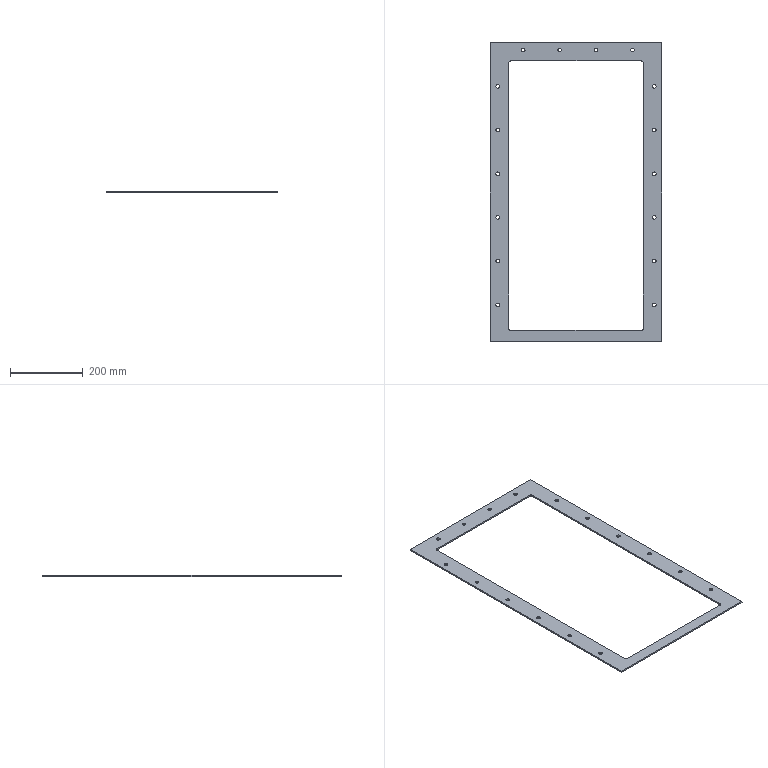Part | SolidWorks | features Fillet 1, FlatPattern 1, ICE 1, SMBaseFlange 1, SheetMetal 1 | 1 solid | 46 faces | box 470 x 820 x 4 mm | volume 441497 mm3 | cylinder 36 | plane 10 | commonest cylinder face diameters 10 x32 12 x4
STEP:
#1=CARTESIAN_POINT('',(25.,60.,-4.));
#2=VERTEX_POINT('',#1);
#3=CARTESIAN_POINT('',(15.,60.,-4.));
#4=VERTEX_POINT('',#3);
#5=CARTESIAN_POINT('',(20.,60.,-4.));
#6=DIRECTION('',(0.,0.,-1.));
#7=DIRECTION('',(-1.,0.,0.));
#8=AXIS2_PLACEMENT_3D('',#5,#6,#7);
#9=CIRCLE('',#8,5.);
#10=EDGE_CURVE('',#2,#4,#9,.T.);
#11=ORIENTED_EDGE('',*,*,#10,.T.);
#12=CARTESIAN_POINT('',(15.,60.,0.));
#13=VERTEX_POINT('',#12);
#14=CARTESIAN_POINT('',(15.,60.,-4.));
#15=DIRECTION('',(0.,0.,1.));
#16=VECTOR('',#15,1000.);
#17=LINE('',#14,#16);
#18=EDGE_CURVE('',#4,#13,#17,.T.);
#19=ORIENTED_EDGE('',*,*,#18,.T.);
#20=CARTESIAN_POINT('',(25.,60.,0.));
#21=VERTEX_POINT('',#20);
#22=CARTESIAN_POINT('',(20.,60.,0.));
#23=DIRECTION('',(0.,0.,-1.));
#24=DIRECTION('',(-1.,0.,0.));
#25=AXIS2_PLACEMENT_3D('',#22,#23,#24);
#26=CIRCLE('',#25,5.);
#27=EDGE_CURVE('',#21,#13,#26,.T.);
#28=ORIENTED_EDGE('',*,*,#27,.F.);
#29=CARTESIAN_POINT('',(25.,60.,-4.));
#30=DIRECTION('',(0.,0.,1.));
#31=VECTOR('',#30,1000.);
#32=LINE('',#29,#31);
#33=EDGE_CURVE('',#2,#21,#32,.T.);
#34=ORIENTED_EDGE('',*,*,#33,.F.);
#35=EDGE_LOOP('',(#11,#19,#28,#34));
#36=FACE_OUTER_BOUND('',#35,.T.);
#37=CARTESIAN_POINT('',(20.,60.,-4.));
#38=DIRECTION('',(0.,0.,1.));
#39=DIRECTION('',(1.,0.,0.));
#40=AXIS2_PLACEMENT_3D('',#37,#38,#39);
#41=CYLINDRICAL_SURFACE('',#40,5.);
#42=ADVANCED_FACE('',(#36),#41,.F.);
#43=CARTESIAN_POINT('',(25.,300.,-4.));
#44=VERTEX_POINT('',#43);
#45=CARTESIAN_POINT('',(15.,300.,-4.));
#46=VERTEX_POINT('',#45);
#47=CARTESIAN_POINT('',(20.,300.,-4.));
#48=DIRECTION('',(0.,0.,-1.));
#49=DIRECTION('',(-1.,0.,0.));
#50=AXIS2_PLACEMENT_3D('',#47,#48,#49);
#51=CIRCLE('',#50,5.);
#52=EDGE_CURVE('',#44,#46,#51,.T.);
#53=ORIENTED_EDGE('',*,*,#52,.T.);
#54=CARTESIAN_POINT('',(15.,300.,0.));
#55=VERTEX_POINT('',#54);
#56=CARTESIAN_POINT('',(15.,300.,-4.));
#57=DIRECTION('',(0.,0.,1.));
#58=VECTOR('',#57,1000.);
#59=LINE('',#56,#58);
#60=EDGE_CURVE('',#46,#55,#59,.T.);
#61=ORIENTED_EDGE('',*,*,#60,.T.);
#62=CARTESIAN_POINT('',(25.,300.,0.));
#63=VERTEX_POINT('',#62);
#64=CARTESIAN_POINT('',(20.,300.,0.));
#65=DIRECTION('',(0.,0.,-1.));
#66=DIRECTION('',(-1.,0.,0.));
#67=AXIS2_PLACEMENT_3D('',#64,#65,#66);
#68=CIRCLE('',#67,5.);
#69=EDGE_CURVE('',#63,#55,#68,.T.);
#70=ORIENTED_EDGE('',*,*,#69,.F.);
#71=CARTESIAN_POINT('',(25.,300.,-4.));
#72=DIRECTION('',(0.,0.,1.));
#73=VECTOR('',#72,1000.);
#74=LINE('',#71,#73);
#75=EDGE_CURVE('',#44,#63,#74,.T.);
#76=ORIENTED_EDGE('',*,*,#75,.F.);
#77=EDGE_LOOP('',(#53,#61,#70,#76));
#78=FACE_OUTER_BOUND('',#77,.T.);
#79=CARTESIAN_POINT('',(20.,300.,-4.));
#80=DIRECTION('',(0.,0.,1.));
#81=DIRECTION('',(1.,0.,0.));
#82=AXIS2_PLACEMENT_3D('',#79,#80,#81);
#83=CYLINDRICAL_SURFACE('',#82,5.);
#84=ADVANCED_FACE('',(#78),#83,.F.);
#85=CARTESIAN_POINT('',(25.,180.,-4.));
#86=VERTEX_POINT('',#85);
#87=CARTESIAN_POINT('',(15.,180.,-4.));
#88=VERTEX_POINT('',#87);
#89=CARTESIAN_POINT('',(20.,180.,-4.));
#90=DIRECTION('',(0.,0.,-1.));
#91=DIRECTION('',(-1.,0.,0.));
#92=AXIS2_PLACEMENT_3D('',#89,#90,#91);
#93=CIRCLE('',#92,5.);
#94=EDGE_CURVE('',#86,#88,#93,.T.);
#95=ORIENTED_EDGE('',*,*,#94,.T.);
#96=CARTESIAN_POINT('',(15.,180.,0.));
#97=VERTEX_POINT('',#96);
#98=CARTESIAN_POINT('',(15.,180.,-4.));
#99=DIRECTION('',(0.,0.,1.));
#100=VECTOR('',#99,1000.);
#101=LINE('',#98,#100);
#102=EDGE_CURVE('',#88,#97,#101,.T.);
#103=ORIENTED_EDGE('',*,*,#102,.T.);
#104=CARTESIAN_POINT('',(25.,180.,0.));
#105=VERTEX_POINT('',#104);
#106=CARTESIAN_POINT('',(20.,180.,0.));
#107=DIRECTION('',(0.,0.,-1.));
#108=DIRECTION('',(-1.,0.,0.));
#109=AXIS2_PLACEMENT_3D('',#106,#107,#108);
#110=CIRCLE('',#109,5.);
#111=EDGE_CURVE('',#105,#97,#110,.T.);
#112=ORIENTED_EDGE('',*,*,#111,.F.);
#113=CARTESIAN_POINT('',(25.,180.,-4.));
#114=DIRECTION('',(0.,0.,1.));
#115=VECTOR('',#114,1000.);
#116=LINE('',#113,#115);
#117=EDGE_CURVE('',#86,#105,#116,.T.);
#118=ORIENTED_EDGE('',*,*,#117,.F.);
#119=EDGE_LOOP('',(#95,#103,#112,#118));
#120=FACE_OUTER_BOUND('',#119,.T.);
#121=CARTESIAN_POINT('',(20.,180.,-4.));
#122=DIRECTION('',(0.,0.,1.));
#123=DIRECTION('',(1.,0.,0.));
#124=AXIS2_PLACEMENT_3D('',#121,#122,#123);
#125=CYLINDRICAL_SURFACE('',#124,5.);
#126=ADVANCED_FACE('',(#120),#125,.F.);
#127=CARTESIAN_POINT('',(25.,-60.,-4.));
#128=VERTEX_POINT('',#127);
#129=CARTESIAN_POINT('',(15.,-60.,-4.));
#130=VERTEX_POINT('',#129);
#131=CARTESIAN_POINT('',(20.,-60.,-4.));
#132=DIRECTION('',(0.,0.,-1.));
#133=DIRECTION('',(-1.,0.,0.));
#134=AXIS2_PLACEMENT_3D('',#131,#132,#133);
#135=CIRCLE('',#134,5.);
#136=EDGE_CURVE('',#128,#130,#135,.T.);
#137=ORIENTED_EDGE('',*,*,#136,.T.);
#138=CARTESIAN_POINT('',(15.,-60.,0.));
#139=VERTEX_POINT('',#138);
#140=CARTESIAN_POINT('',(15.,-60.,-4.));
#141=DIRECTION('',(0.,0.,1.));
#142=VECTOR('',#141,1000.);
#143=LINE('',#140,#142);
#144=EDGE_CURVE('',#130,#139,#143,.T.);
#145=ORIENTED_EDGE('',*,*,#144,.T.);
#146=CARTESIAN_POINT('',(25.,-60.,0.));
#147=VERTEX_POINT('',#146);
#148=CARTESIAN_POINT('',(20.,-60.,0.));
#149=DIRECTION('',(0.,0.,-1.));
#150=DIRECTION('',(-1.,0.,0.));
#151=AXIS2_PLACEMENT_3D('',#148,#149,#150);
#152=CIRCLE('',#151,5.);
#153=EDGE_CURVE('',#147,#139,#152,.T.);
#154=ORIENTED_EDGE('',*,*,#153,.F.);
#155=CARTESIAN_POINT('',(25.,-60.,-4.));
#156=DIRECTION('',(0.,0.,1.));
#157=VECTOR('',#156,1000.);
#158=LINE('',#155,#157);
#159=EDGE_CURVE('',#128,#147,#158,.T.);
#160=ORIENTED_EDGE('',*,*,#159,.F.);
#161=EDGE_LOOP('',(#137,#145,#154,#160));
#162=FACE_OUTER_BOUND('',#161,.T.);
#163=CARTESIAN_POINT('',(20.,-60.,-4.));
#164=DIRECTION('',(0.,0.,1.));
#165=DIRECTION('',(1.,0.,0.));
#166=AXIS2_PLACEMENT_3D('',#163,#164,#165);
#167=CYLINDRICAL_SURFACE('',#166,5.);
#168=ADVANCED_FACE('',(#162),#167,.F.);
#169=CARTESIAN_POINT('',(25.,-180.,-4.));
#170=VERTEX_POINT('',#169);
#171=CARTESIAN_POINT('',(15.,-180.,-4.));
#172=VERTEX_POINT('',#171);
#173=CARTESIAN_POINT('',(20.,-180.,-4.));
#174=DIRECTION('',(0.,0.,-1.));
#175=DIRECTION('',(-1.,0.,0.));
#176=AXIS2_PLACEMENT_3D('',#173,#174,#175);
#177=CIRCLE('',#176,5.);
#178=EDGE_CURVE('',#170,#172,#177,.T.);
#179=ORIENTED_EDGE('',*,*,#178,.T.);
#180=CARTESIAN_POINT('',(15.,-180.,0.));
#181=VERTEX_POINT('',#180);
#182=CARTESIAN_POINT('',(15.,-180.,-4.));
#183=DIRECTION('',(0.,0.,1.));
#184=VECTOR('',#183,1000.);
#185=LINE('',#182,#184);
#186=EDGE_CURVE('',#172,#181,#185,.T.);
#187=ORIENTED_EDGE('',*,*,#186,.T.);
#188=CARTESIAN_POINT('',(25.,-180.,0.));
#189=VERTEX_POINT('',#188);
#190=CARTESIAN_POINT('',(20.,-180.,0.));
#191=DIRECTION('',(0.,0.,-1.));
#192=DIRECTION('',(-1.,0.,0.));
#193=AXIS2_PLACEMENT_3D('',#190,#191,#192);
#194=CIRCLE('',#193,5.);
#195=EDGE_CURVE('',#189,#181,#194,.T.);
#196=ORIENTED_EDGE('',*,*,#195,.F.);
#197=CARTESIAN_POINT('',(25.,-180.,-4.));
#198=DIRECTION('',(0.,0.,1.));
#199=VECTOR('',#198,1000.);
#200=LINE('',#197,#199);
#201=EDGE_CURVE('',#170,#189,#200,.T.);
#202=ORIENTED_EDGE('',*,*,#201,.F.);
#203=EDGE_LOOP('',(#179,#187,#196,#202));
#204=FACE_OUTER_BOUND('',#203,.T.);
#205=CARTESIAN_POINT('',(20.,-180.,-4.));
#206=DIRECTION('',(0.,0.,1.));
#207=DIRECTION('',(1.,0.,0.));
#208=AXIS2_PLACEMENT_3D('',#205,#206,#207);
#209=CYLINDRICAL_SURFACE('',#208,5.);
#210=ADVANCED_FACE('',(#204),#209,.F.);
#211=CARTESIAN_POINT('',(25.,-300.,-4.));
#212=VERTEX_POINT('',#211);
#213=CARTESIAN_POINT('',(15.,-300.,-4.));
#214=VERTEX_POINT('',#213);
#215=CARTESIAN_POINT('',(20.,-300.,-4.));
#216=DIRECTION('',(0.,0.,-1.));
#217=DIRECTION('',(-1.,0.,0.));
#218=AXIS2_PLACEMENT_3D('',#215,#216,#217);
#219=CIRCLE('',#218,5.);
#220=EDGE_CURVE('',#212,#214,#219,.T.);
#221=ORIENTED_EDGE('',*,*,#220,.T.);
#222=CARTESIAN_POINT('',(15.,-300.,0.));
#223=VERTEX_POINT('',#222);
#224=CARTESIAN_POINT('',(15.,-300.,-4.));
#225=DIRECTION('',(0.,0.,1.));
#226=VECTOR('',#225,1000.);
#227=LINE('',#224,#226);
#228=EDGE_CURVE('',#214,#223,#227,.T.);
#229=ORIENTED_EDGE('',*,*,#228,.T.);
#230=CARTESIAN_POINT('',(25.,-300.,0.));
#231=VERTEX_POINT('',#230);
#232=CARTESIAN_POINT('',(20.,-300.,0.));
#233=DIRECTION('',(0.,0.,-1.));
#234=DIRECTION('',(-1.,0.,0.));
#235=AXIS2_PLACEMENT_3D('',#232,#233,#234);
#236=CIRCLE('',#235,5.);
#237=EDGE_CURVE('',#231,#223,#236,.T.);
#238=ORIENTED_EDGE('',*,*,#237,.F.);
#239=CARTESIAN_POINT('',(25.,-300.,-4.));
#240=DIRECTION('',(0.,0.,1.));
#241=VECTOR('',#240,1000.);
#242=LINE('',#239,#241);
#243=EDGE_CURVE('',#212,#231,#242,.T.);
#244=ORIENTED_EDGE('',*,*,#243,.F.);
#245=EDGE_LOOP('',(#221,#229,#238,#244));
#246=FACE_OUTER_BOUND('',#245,.T.);
#247=CARTESIAN_POINT('',(20.,-300.,-4.));
#248=DIRECTION('',(0.,0.,1.));
#249=DIRECTION('',(1.,0.,0.));
#250=AXIS2_PLACEMENT_3D('',#247,#248,#249);
#251=CYLINDRICAL_SURFACE('',#250,5.);
#252=ADVANCED_FACE('',(#246),#251,.F.);
#253=CARTESIAN_POINT('',(-415.,-300.,-4.));
#254=VERTEX_POINT('',#253);
#255=CARTESIAN_POINT('',(-405.,-300.,-4.));
#256=VERTEX_POINT('',#255);
#257=CARTESIAN_POINT('',(-410.,-300.,-4.));
#258=DIRECTION('',(0.,0.,1.));
#259=DIRECTION('',(1.,0.,0.));
#260=AXIS2_PLACEMENT_3D('',#257,#258,#259);
#261=CIRCLE('',#260,5.);
#262=EDGE_CURVE('',#254,#256,#261,.T.);
#263=ORIENTED_EDGE('',*,*,#262,.F.);
#264=CARTESIAN_POINT('',(-415.,-300.,0.));
#265=VERTEX_POINT('',#264);
#266=CARTESIAN_POINT('',(-415.,-300.,-4.));
#267=DIRECTION('',(0.,0.,1.));
#268=VECTOR('',#267,1000.);
#269=LINE('',#266,#268);
#270=EDGE_CURVE('',#254,#265,#269,.T.);
#271=ORIENTED_EDGE('',*,*,#270,.T.);
#272=CARTESIAN_POINT('',(-405.,-300.,0.));
#273=VERTEX_POINT('',#272);
#274=CARTESIAN_POINT('',(-410.,-300.,0.));
#275=DIRECTION('',(0.,0.,1.));
#276=DIRECTION('',(1.,0.,0.));
#277=AXIS2_PLACEMENT_3D('',#274,#275,#276);
#278=CIRCLE('',#277,5.);
#279=EDGE_CURVE('',#265,#273,#278,.T.);
#280=ORIENTED_EDGE('',*,*,#279,.T.);
#281=CARTESIAN_POINT('',(-405.,-300.,-4.));
#282=DIRECTION('',(0.,0.,1.));
#283=VECTOR('',#282,1000.);
#284=LINE('',#281,#283);
#285=EDGE_CURVE('',#256,#273,#284,.T.);
#286=ORIENTED_EDGE('',*,*,#285,.F.);
#287=EDGE_LOOP('',(#263,#271,#280,#286));
#288=FACE_OUTER_BOUND('',#287,.T.);
#289=CARTESIAN_POINT('',(-410.,-300.,-4.));
#290=DIRECTION('',(0.,0.,1.));
#291=DIRECTION('',(1.,0.,0.));
#292=AXIS2_PLACEMENT_3D('',#289,#290,#291);
#293=CYLINDRICAL_SURFACE('',#292,5.);
#294=ADVANCED_FACE('',(#288),#293,.F.);
#295=CARTESIAN_POINT('',(-415.,-180.,-4.));
#296=VERTEX_POINT('',#295);
#297=CARTESIAN_POINT('',(-405.,-180.,-4.));
#298=VERTEX_POINT('',#297);
#299=CARTESIAN_POINT('',(-410.,-180.,-4.));
#300=DIRECTION('',(0.,0.,1.));
#301=DIRECTION('',(1.,0.,0.));
#302=AXIS2_PLACEMENT_3D('',#299,#300,#301);
#303=CIRCLE('',#302,5.);
#304=EDGE_CURVE('',#296,#298,#303,.T.);
#305=ORIENTED_EDGE('',*,*,#304,.F.);
#306=CARTESIAN_POINT('',(-415.,-180.,0.));
#307=VERTEX_POINT('',#306);
#308=CARTESIAN_POINT('',(-415.,-180.,-4.));
#309=DIRECTION('',(0.,0.,1.));
#310=VECTOR('',#309,1000.);
#311=LINE('',#308,#310);
#312=EDGE_CURVE('',#296,#307,#311,.T.);
#313=ORIENTED_EDGE('',*,*,#312,.T.);
#314=CARTESIAN_POINT('',(-405.,-180.,0.));
#315=VERTEX_POINT('',#314);
#316=CARTESIAN_POINT('',(-410.,-180.,0.));
#317=DIRECTION('',(0.,0.,1.));
#318=DIRECTION('',(1.,0.,0.));
#319=AXIS2_PLACEMENT_3D('',#316,#317,#318);
#320=CIRCLE('',#319,5.);
#321=EDGE_CURVE('',#307,#315,#320,.T.);
#322=ORIENTED_EDGE('',*,*,#321,.T.);
#323=CARTESIAN_POINT('',(-405.,-180.,-4.));
#324=DIRECTION('',(0.,0.,1.));
#325=VECTOR('',#324,1000.);
#326=LINE('',#323,#325);
#327=EDGE_CURVE('',#298,#315,#326,.T.);
#328=ORIENTED_EDGE('',*,*,#327,.F.);
#329=EDGE_LOOP('',(#305,#313,#322,#328));
#330=FACE_OUTER_BOUND('',#329,.T.);
#331=CARTESIAN_POINT('',(-410.,-180.,-4.));
#332=DIRECTION('',(0.,0.,1.));
#333=DIRECTION('',(1.,0.,0.));
#334=AXIS2_PLACEMENT_3D('',#331,#332,#333);
#335=CYLINDRICAL_SURFACE('',#334,5.);
#336=ADVANCED_FACE('',(#330),#335,.F.);
#337=CARTESIAN_POINT('',(-415.,-60.,-4.));
#338=VERTEX_POINT('',#337);
#339=CARTESIAN_POINT('',(-405.,-60.,-4.));
#340=VERTEX_POINT('',#339);
#341=CARTESIAN_POINT('',(-410.,-60.,-4.));
#342=DIRECTION('',(0.,0.,1.));
#343=DIRECTION('',(1.,0.,0.));
#344=AXIS2_PLACEMENT_3D('',#341,#342,#343);
#345=CIRCLE('',#344,5.);
#346=EDGE_CURVE('',#338,#340,#345,.T.);
#347=ORIENTED_EDGE('',*,*,#346,.F.);
#348=CARTESIAN_POINT('',(-415.,-60.,0.));
#349=VERTEX_POINT('',#348);
#350=CARTESIAN_POINT('',(-415.,-60.,-4.));
#351=DIRECTION('',(0.,0.,1.));
#352=VECTOR('',#351,1000.);
#353=LINE('',#350,#352);
#354=EDGE_CURVE('',#338,#349,#353,.T.);
#355=ORIENTED_EDGE('',*,*,#354,.T.);
#356=CARTESIAN_POINT('',(-405.,-60.,0.));
#357=VERTEX_POINT('',#356);
#358=CARTESIAN_POINT('',(-410.,-60.,0.));
#359=DIRECTION('',(0.,0.,1.));
#360=DIRECTION('',(1.,0.,0.));
#361=AXIS2_PLACEMENT_3D('',#358,#359,#360);
#362=CIRCLE('',#361,5.);
#363=EDGE_CURVE('',#349,#357,#362,.T.);
#364=ORIENTED_EDGE('',*,*,#363,.T.);
#365=CARTESIAN_POINT('',(-405.,-60.,-4.));
#366=DIRECTION('',(0.,0.,1.));
#367=VECTOR('',#366,1000.);
#368=LINE('',#365,#367);
#369=EDGE_CURVE('',#340,#357,#368,.T.);
#370=ORIENTED_EDGE('',*,*,#369,.F.);
#371=EDGE_LOOP('',(#347,#355,#364,#370));
#372=FACE_OUTER_BOUND('',#371,.T.);
#373=CARTESIAN_POINT('',(-410.,-60.,-4.));
#374=DIRECTION('',(0.,0.,1.));
#375=DIRECTION('',(1.,0.,0.));
#376=AXIS2_PLACEMENT_3D('',#373,#374,#375);
#377=CYLINDRICAL_SURFACE('',#376,5.);
#378=ADVANCED_FACE('',(#372),#377,.F.);
#379=CARTESIAN_POINT('',(-415.,60.,-4.));
#380=VERTEX_POINT('',#379);
#381=CARTESIAN_POINT('',(-405.,60.,-4.));
#382=VERTEX_POINT('',#381);
#383=CARTESIAN_POINT('',(-410.,60.,-4.));
#384=DIRECTION('',(0.,0.,1.));
#385=DIRECTION('',(1.,0.,0.));
#386=AXIS2_PLACEMENT_3D('',#383,#384,#385);
#387=CIRCLE('',#386,5.);
#388=EDGE_CURVE('',#380,#382,#387,.T.);
#389=ORIENTED_EDGE('',*,*,#388,.F.);
#390=CARTESIAN_POINT('',(-415.,60.,0.));
#391=VERTEX_POINT('',#390);
#392=CARTESIAN_POINT('',(-415.,60.,-4.));
#393=DIRECTION('',(0.,0.,1.));
#394=VECTOR('',#393,1000.);
#395=LINE('',#392,#394);
#396=EDGE_CURVE('',#380,#391,#395,.T.);
#397=ORIENTED_EDGE('',*,*,#396,.T.);
#398=CARTESIAN_POINT('',(-405.,60.,0.));
#399=VERTEX_POINT('',#398);
#400=CARTESIAN_POINT('',(-410.,60.,0.));
#401=DIRECTION('',(0.,0.,1.));
#402=DIRECTION('',(1.,0.,0.));
#403=AXIS2_PLACEMENT_3D('',#400,#401,#402);
#404=CIRCLE('',#403,5.);
#405=EDGE_CURVE('',#391,#399,#404,.T.);
#406=ORIENTED_EDGE('',*,*,#405,.T.);
#407=CARTESIAN_POINT('',(-405.,60.,-4.));
#408=DIRECTION('',(0.,0.,1.));
#409=VECTOR('',#408,1000.);
#410=LINE('',#407,#409);
#411=EDGE_CURVE('',#382,#399,#410,.T.);
#412=ORIENTED_EDGE('',*,*,#411,.F.);
#413=EDGE_LOOP('',(#389,#397,#406,#412));
#414=FACE_OUTER_BOUND('',#413,.T.);
#415=CARTESIAN_POINT('',(-410.,60.,-4.));
#416=DIRECTION('',(0.,0.,1.));
#417=DIRECTION('',(1.,0.,0.));
#418=AXIS2_PLACEMENT_3D('',#415,#416,#417);
#419=CYLINDRICAL_SURFACE('',#418,5.);
#420=ADVANCED_FACE('',(#414),#419,.F.);
#421=CARTESIAN_POINT('',(-415.,180.,-4.));
#422=VERTEX_POINT('',#421);
#423=CARTESIAN_POINT('',(-405.,180.,-4.));
#424=VERTEX_POINT('',#423);
#425=CARTESIAN_POINT('',(-410.,180.,-4.));
#426=DIRECTION('',(0.,0.,1.));
#427=DIRECTION('',(1.,0.,0.));
#428=AXIS2_PLACEMENT_3D('',#425,#426,#427);
#429=CIRCLE('',#428,5.);
#430=EDGE_CURVE('',#422,#424,#429,.T.);
#431=ORIENTED_EDGE('',*,*,#430,.F.);
#432=CARTESIAN_POINT('',(-415.,180.,0.));
#433=VERTEX_POINT('',#432);
#434=CARTESIAN_POINT('',(-415.,180.,-4.));
#435=DIRECTION('',(0.,0.,1.));
#436=VECTOR('',#435,1000.);
#437=LINE('',#434,#436);
#438=EDGE_CURVE('',#422,#433,#437,.T.);
#439=ORIENTED_EDGE('',*,*,#438,.T.);
#440=CARTESIAN_POINT('',(-405.,180.,0.));
#441=VERTEX_POINT('',#440);
#442=CARTESIAN_POINT('',(-410.,180.,0.));
#443=DIRECTION('',(0.,0.,1.));
#444=DIRECTION('',(1.,0.,0.));
#445=AXIS2_PLACEMENT_3D('',#442,#443,#444);
#446=CIRCLE('',#445,5.);
#447=EDGE_CURVE('',#433,#441,#446,.T.);
#448=ORIENTED_EDGE('',*,*,#447,.T.);
#449=CARTESIAN_POINT('',(-405.,180.,-4.));
#450=DIRECTION('',(0.,0.,1.));
#451=VECTOR('',#450,1000.);
#452=LINE('',#449,#451);
#453=EDGE_CURVE('',#424,#441,#452,.T.);
#454=ORIENTED_EDGE('',*,*,#453,.F.);
#455=EDGE_LOOP('',(#431,#439,#448,#454));
#456=FACE_OUTER_BOUND('',#455,.T.);
#457=CARTESIAN_POINT('',(-410.,180.,-4.));
#458=DIRECTION('',(0.,0.,1.));
#459=DIRECTION('',(1.,0.,0.));
#460=AXIS2_PLACEMENT_3D('',#457,#458,#459);
#461=CYLINDRICAL_SURFACE('',#460,5.);
#462=ADVANCED_FACE('',(#456),#461,.F.);
#463=CARTESIAN_POINT('',(-415.,300.,-4.));
#464=VERTEX_POINT('',#463);
#465=CARTESIAN_POINT('',(-405.,300.,-4.));
#466=VERTEX_POINT('',#465);
#467=CARTESIAN_POINT('',(-410.,300.,-4.));
#468=DIRECTION('',(0.,0.,1.));
#469=DIRECTION('',(1.,0.,0.));
#470=AXIS2_PLACEMENT_3D('',#467,#468,#469);
#471=CIRCLE('',#470,5.);
#472=EDGE_CURVE('',#464,#466,#471,.T.);
#473=ORIENTED_EDGE('',*,*,#472,.F.);
#474=CARTESIAN_POINT('',(-415.,300.,0.));
#475=VERTEX_POINT('',#474);
#476=CARTESIAN_POINT('',(-415.,300.,-4.));
#477=DIRECTION('',(0.,0.,1.));
#478=VECTOR('',#477,1000.);
#479=LINE('',#476,#478);
#480=EDGE_CURVE('',#464,#475,#479,.T.);
#481=ORIENTED_EDGE('',*,*,#480,.T.);
#482=CARTESIAN_POINT('',(-405.,300.,0.));
#483=VERTEX_POINT('',#482);
#484=CARTESIAN_POINT('',(-410.,300.,0.));
#485=DIRECTION('',(0.,0.,1.));
#486=DIRECTION('',(1.,0.,0.));
#487=AXIS2_PLACEMENT_3D('',#484,#485,#486);
#488=CIRCLE('',#487,5.);
#489=EDGE_CURVE('',#475,#483,#488,.T.);
#490=ORIENTED_EDGE('',*,*,#489,.T.);
#491=CARTESIAN_POINT('',(-405.,300.,-4.));
#492=DIRECTION('',(0.,0.,1.));
#493=VECTOR('',#492,1000.);
#494=LINE('',#491,#493);
#495=EDGE_CURVE('',#466,#483,#494,.T.);
#496=ORIENTED_EDGE('',*,*,#495,.F.);
#497=EDGE_LOOP('',(#473,#481,#490,#496));
#498=FACE_OUTER_BOUND('',#497,.T.);
#499=CARTESIAN_POINT('',(-410.,300.,-4.));
#500=DIRECTION('',(0.,0.,1.));
#501=DIRECTION('',(1.,0.,0.));
#502=AXIS2_PLACEMENT_3D('',#499,#500,#501);
#503=CYLINDRICAL_SURFACE('',#502,5.);
#504=ADVANCED_FACE('',(#498),#503,.F.);
#505=CARTESIAN_POINT('',(-45.,400.,-4.));
#506=VERTEX_POINT('',#505);
#507=CARTESIAN_POINT('',(-35.,400.,-4.));
#508=VERTEX_POINT('',#507);
#509=CARTESIAN_POINT('',(-40.,400.,-4.));
#510=DIRECTION('',(0.,0.,1.));
#511=DIRECTION('',(1.,0.,0.));
#512=AXIS2_PLACEMENT_3D('',#509,#510,#511);
#513=CIRCLE('',#512,5.);
#514=EDGE_CURVE('',#506,#508,#513,.T.);
#515=ORIENTED_EDGE('',*,*,#514,.F.);
#516=CARTESIAN_POINT('',(-45.,400.,0.));
#517=VERTEX_POINT('',#516);
#518=CARTESIAN_POINT('',(-45.,400.,-4.));
#519=DIRECTION('',(0.,0.,1.));
#520=VECTOR('',#519,1000.);
#521=LINE('',#518,#520);
#522=EDGE_CURVE('',#506,#517,#521,.T.);
#523=ORIENTED_EDGE('',*,*,#522,.T.);
#524=CARTESIAN_POINT('',(-35.,400.,0.));
#525=VERTEX_POINT('',#524);
#526=CARTESIAN_POINT('',(-40.,400.,0.));
#527=DIRECTION('',(0.,0.,1.));
#528=DIRECTION('',(1.,0.,0.));
#529=AXIS2_PLACEMENT_3D('',#526,#527,#528);
#530=CIRCLE('',#529,5.);
#531=EDGE_CURVE('',#517,#525,#530,.T.);
#532=ORIENTED_EDGE('',*,*,#531,.T.);
#533=CARTESIAN_POINT('',(-35.,400.,-4.));
#534=DIRECTION('',(0.,0.,1.));
#535=VECTOR('',#534,1000.);
#536=LINE('',#533,#535);
#537=EDGE_CURVE('',#508,#525,#536,.T.);
#538=ORIENTED_EDGE('',*,*,#537,.F.);
#539=EDGE_LOOP('',(#515,#523,#532,#538));
#540=FACE_OUTER_BOUND('',#539,.T.);
#541=CARTESIAN_POINT('',(-40.,400.,-4.));
#542=DIRECTION('',(0.,0.,1.));
#543=DIRECTION('',(1.,0.,0.));
#544=AXIS2_PLACEMENT_3D('',#541,#542,#543);
#545=CYLINDRICAL_SURFACE('',#544,5.);
#546=ADVANCED_FACE('',(#540),#545,.F.);
#547=CARTESIAN_POINT('',(-145.,400.,-4.));
#548=VERTEX_POINT('',#547);
#549=CARTESIAN_POINT('',(-135.,400.,-4.));
#550=VERTEX_POINT('',#549);
#551=CARTESIAN_POINT('',(-140.,400.,-4.));
#552=DIRECTION('',(0.,0.,1.));
#553=DIRECTION('',(1.,0.,0.));
#554=AXIS2_PLACEMENT_3D('',#551,#552,#553);
#555=CIRCLE('',#554,5.);
#556=EDGE_CURVE('',#548,#550,#555,.T.);
#557=ORIENTED_EDGE('',*,*,#556,.F.);
#558=CARTESIAN_POINT('',(-145.,400.,0.));
#559=VERTEX_POINT('',#558);
#560=CARTESIAN_POINT('',(-145.,400.,-4.));
#561=DIRECTION('',(0.,0.,1.));
#562=VECTOR('',#561,1000.);
#563=LINE('',#560,#562);
#564=EDGE_CURVE('',#548,#559,#563,.T.);
#565=ORIENTED_EDGE('',*,*,#564,.T.);
#566=CARTESIAN_POINT('',(-135.,400.,0.));
#567=VERTEX_POINT('',#566);
#568=CARTESIAN_POINT('',(-140.,400.,0.));
#569=DIRECTION('',(0.,0.,1.));
#570=DIRECTION('',(1.,0.,0.));
#571=AXIS2_PLACEMENT_3D('',#568,#569,#570);
#572=CIRCLE('',#571,5.);
#573=EDGE_CURVE('',#559,#567,#572,.T.);
#574=ORIENTED_EDGE('',*,*,#573,.T.);
#575=CARTESIAN_POINT('',(-135.,400.,-4.));
#576=DIRECTION('',(0.,0.,1.));
#577=VECTOR('',#576,1000.);
#578=LINE('',#575,#577);
#579=EDGE_CURVE('',#550,#567,#578,.T.);
#580=ORIENTED_EDGE('',*,*,#579,.F.);
#581=EDGE_LOOP('',(#557,#565,#574,#580));
#582=FACE_OUTER_BOUND('',#581,.T.);
#583=CARTESIAN_POINT('',(-140.,400.,-4.));
#584=DIRECTION('',(0.,0.,1.));
#585=DIRECTION('',(1.,0.,0.));
#586=AXIS2_PLACEMENT_3D('',#583,#584,#585);
#587=CYLINDRICAL_SURFACE('',#586,5.);
#588=ADVANCED_FACE('',(#582),#587,.F.);
#589=CARTESIAN_POINT('',(-245.,400.,-4.));
#590=VERTEX_POINT('',#589);
#591=CARTESIAN_POINT('',(-235.,400.,-4.));
#592=VERTEX_POINT('',#591);
#593=CARTESIAN_POINT('',(-240.,400.,-4.));
#594=DIRECTION('',(0.,0.,1.));
#595=DIRECTION('',(1.,0.,0.));
#596=AXIS2_PLACEMENT_3D('',#593,#594,#595);
#597=CIRCLE('',#596,5.);
#598=EDGE_CURVE('',#590,#592,#597,.T.);
#599=ORIENTED_EDGE('',*,*,#598,.F.);
#600=CARTESIAN_POINT('',(-245.,400.,0.));
#601=VERTEX_POINT('',#600);
#602=CARTESIAN_POINT('',(-245.,400.,-4.));
#603=DIRECTION('',(0.,0.,1.));
#604=VECTOR('',#603,1000.);
#605=LINE('',#602,#604);
#606=EDGE_CURVE('',#590,#601,#605,.T.);
#607=ORIENTED_EDGE('',*,*,#606,.T.);
#608=CARTESIAN_POINT('',(-235.,400.,0.));
#609=VERTEX_POINT('',#608);
#610=CARTESIAN_POINT('',(-240.,400.,0.));
#611=DIRECTION('',(0.,0.,1.));
#612=DIRECTION('',(1.,0.,0.));
#613=AXIS2_PLACEMENT_3D('',#610,#611,#612);
#614=CIRCLE('',#613,5.);
#615=EDGE_CURVE('',#601,#609,#614,.T.);
#616=ORIENTED_EDGE('',*,*,#615,.T.);
#617=CARTESIAN_POINT('',(-235.,400.,-4.));
#618=DIRECTION('',(0.,0.,1.));
#619=VECTOR('',#618,1000.);
#620=LINE('',#617,#619);
#621=EDGE_CURVE('',#592,#609,#620,.T.);
#622=ORIENTED_EDGE('',*,*,#621,.F.);
#623=EDGE_LOOP('',(#599,#607,#616,#622));
#624=FACE_OUTER_BOUND('',#623,.T.);
#625=CARTESIAN_POINT('',(-240.,400.,-4.));
#626=DIRECTION('',(0.,0.,1.));
#627=DIRECTION('',(1.,0.,0.));
#628=AXIS2_PLACEMENT_3D('',#625,#626,#627);
#629=CYLINDRICAL_SURFACE('',#628,5.);
#630=ADVANCED_FACE('',(#624),#629,.F.);
#631=CARTESIAN_POINT('',(-345.,400.,-4.));
#632=VERTEX_POINT('',#631);
#633=CARTESIAN_POINT('',(-335.,400.,-4.));
#634=VERTEX_POINT('',#633);
#635=CARTESIAN_POINT('',(-340.,400.,-4.));
#636=DIRECTION('',(0.,0.,1.));
#637=DIRECTION('',(1.,0.,0.));
#638=AXIS2_PLACEMENT_3D('',#635,#636,#637);
#639=CIRCLE('',#638,5.);
#640=EDGE_CURVE('',#632,#634,#639,.T.);
#641=ORIENTED_EDGE('',*,*,#640,.F.);
#642=CARTESIAN_POINT('',(-345.,400.,0.));
#643=VERTEX_POINT('',#642);
#644=CARTESIAN_POINT('',(-345.,400.,-4.));
#645=DIRECTION('',(0.,0.,1.));
#646=VECTOR('',#645,1000.);
#647=LINE('',#644,#646);
#648=EDGE_CURVE('',#632,#643,#647,.T.);
#649=ORIENTED_EDGE('',*,*,#648,.T.);
#650=CARTESIAN_POINT('',(-335.,400.,0.));
#651=VERTEX_POINT('',#650);
#652=CARTESIAN_POINT('',(-340.,400.,0.));
#653=DIRECTION('',(0.,0.,1.));
#654=DIRECTION('',(1.,0.,0.));
#655=AXIS2_PLACEMENT_3D('',#652,#653,#654);
#656=CIRCLE('',#655,5.);
#657=EDGE_CURVE('',#643,#651,#656,.T.);
#658=ORIENTED_EDGE('',*,*,#657,.T.);
#659=CARTESIAN_POINT('',(-335.,400.,-4.));
#660=DIRECTION('',(0.,0.,1.));
#661=VECTOR('',#660,1000.);
#662=LINE('',#659,#661);
#663=EDGE_CURVE('',#634,#651,#662,.T.);
#664=ORIENTED_EDGE('',*,*,#663,.F.);
#665=EDGE_LOOP('',(#641,#649,#658,#664));
#666=FACE_OUTER_BOUND('',#665,.T.);
#667=CARTESIAN_POINT('',(-340.,400.,-4.));
#668=DIRECTION('',(0.,0.,1.));
#669=DIRECTION('',(1.,0.,0.));
#670=AXIS2_PLACEMENT_3D('',#667,#668,#669);
#671=CYLINDRICAL_SURFACE('',#670,5.);
#672=ADVANCED_FACE('',(#666),#671,.F.);
#673=CARTESIAN_POINT('',(-410.,-300.,-4.));
#674=DIRECTION('',(0.,0.,1.));
#675=DIRECTION('',(1.,0.,0.));
#676=AXIS2_PLACEMENT_3D('',#673,#674,#675);
#677=CIRCLE('',#676,5.);
#678=EDGE_CURVE('',#256,#254,#677,.T.);
#679=ORIENTED_EDGE('',*,*,#678,.T.);
#680=ORIENTED_EDGE('',*,*,#262,.T.);
#681=EDGE_LOOP('',(#679,#680));
#682=FACE_BOUND('',#681,.T.);
#683=CARTESIAN_POINT('',(-410.,-180.,-4.));
#684=DIRECTION('',(0.,0.,1.));
#685=DIRECTION('',(1.,0.,0.));
#686=AXIS2_PLACEMENT_3D('',#683,#684,#685);
#687=CIRCLE('',#686,5.);
#688=EDGE_CURVE('',#298,#296,#687,.T.);
#689=ORIENTED_EDGE('',*,*,#688,.T.);
#690=ORIENTED_EDGE('',*,*,#304,.T.);
#691=EDGE_LOOP('',(#689,#690));
#692=FACE_BOUND('',#691,.T.);
#693=CARTESIAN_POINT('',(-410.,-60.,-4.));
#694=DIRECTION('',(0.,0.,1.));
#695=DIRECTION('',(1.,0.,0.));
#696=AXIS2_PLACEMENT_3D('',#693,#694,#695);
#697=CIRCLE('',#696,5.);
#698=EDGE_CURVE('',#340,#338,#697,.T.);
#699=ORIENTED_EDGE('',*,*,#698,.T.);
#700=ORIENTED_EDGE('',*,*,#346,.T.);
#701=EDGE_LOOP('',(#699,#700));
#702=FACE_BOUND('',#701,.T.);
#703=CARTESIAN_POINT('',(-410.,60.,-4.));
#704=DIRECTION('',(0.,0.,1.));
#705=DIRECTION('',(1.,0.,0.));
#706=AXIS2_PLACEMENT_3D('',#703,#704,#705);
#707=CIRCLE('',#706,5.);
#708=EDGE_CURVE('',#382,#380,#707,.T.);
#709=ORIENTED_EDGE('',*,*,#708,.T.);
#710=ORIENTED_EDGE('',*,*,#388,.T.);
#711=EDGE_LOOP('',(#709,#710));
#712=FACE_BOUND('',#711,.T.);
#713=CARTESIAN_POINT('',(-410.,180.,-4.));
#714=DIRECTION('',(0.,0.,1.));
#715=DIRECTION('',(1.,0.,0.));
#716=AXIS2_PLACEMENT_3D('',#713,#714,#715);
#717=CIRCLE('',#716,5.);
#718=EDGE_CURVE('',#424,#422,#717,.T.);
#719=ORIENTED_EDGE('',*,*,#718,.T.);
#720=ORIENTED_EDGE('',*,*,#430,.T.);
#721=EDGE_LOOP('',(#719,#720));
#722=FACE_BOUND('',#721,.T.);
#723=CARTESIAN_POINT('',(-410.,300.,-4.));
#724=DIRECTION('',(0.,0.,1.));
#725=DIRECTION('',(1.,0.,0.));
#726=AXIS2_PLACEMENT_3D('',#723,#724,#725);
#727=CIRCLE('',#726,5.);
#728=EDGE_CURVE('',#466,#464,#727,.T.);
#729=ORIENTED_EDGE('',*,*,#728,.T.);
#730=ORIENTED_EDGE('',*,*,#472,.T.);
#731=EDGE_LOOP('',(#729,#730));
#732=FACE_BOUND('',#731,.T.);
#733=CARTESIAN_POINT('',(-40.,400.,-4.));
#734=DIRECTION('',(0.,0.,1.));
#735=DIRECTION('',(1.,0.,0.));
#736=AXIS2_PLACEMENT_3D('',#733,#734,#735);
#737=CIRCLE('',#736,5.);
#738=EDGE_CURVE('',#508,#506,#737,.T.);
#739=ORIENTED_EDGE('',*,*,#738,.T.);
#740=ORIENTED_EDGE('',*,*,#514,.T.);
#741=EDGE_LOOP('',(#739,#740));
#742=FACE_BOUND('',#741,.T.);
#743=CARTESIAN_POINT('',(-140.,400.,-4.));
#744=DIRECTION('',(0.,0.,1.));
#745=DIRECTION('',(1.,0.,0.));
#746=AXIS2_PLACEMENT_3D('',#743,#744,#745);
#747=CIRCLE('',#746,5.);
#748=EDGE_CURVE('',#550,#548,#747,.T.);
#749=ORIENTED_EDGE('',*,*,#748,.T.);
#750=ORIENTED_EDGE('',*,*,#556,.T.);
#751=EDGE_LOOP('',(#749,#750));
#752=FACE_BOUND('',#751,.T.);
#753=CARTESIAN_POINT('',(-240.,400.,-4.));
#754=DIRECTION('',(0.,0.,1.));
#755=DIRECTION('',(1.,0.,0.));
#756=AXIS2_PLACEMENT_3D('',#753,#754,#755);
#757=CIRCLE('',#756,5.);
#758=EDGE_CURVE('',#592,#590,#757,.T.);
#759=ORIENTED_EDGE('',*,*,#758,.T.);
#760=ORIENTED_EDGE('',*,*,#598,.T.);
#761=EDGE_LOOP('',(#759,#760));
#762=FACE_BOUND('',#761,.T.);
#763=CARTESIAN_POINT('',(-340.,400.,-4.));
#764=DIRECTION('',(0.,0.,1.));
#765=DIRECTION('',(1.,0.,0.));
#766=AXIS2_PLACEMENT_3D('',#763,#764,#765);
#767=CIRCLE('',#766,5.);
#768=EDGE_CURVE('',#634,#632,#767,.T.);
#769=ORIENTED_EDGE('',*,*,#768,.T.);
#770=ORIENTED_EDGE('',*,*,#640,.T.);
#771=EDGE_LOOP('',(#769,#770));
#772=FACE_BOUND('',#771,.T.);
#773=CARTESIAN_POINT('',(40.,420.,-4.));
#774=VERTEX_POINT('',#773);
#775=CARTESIAN_POINT('',(40.,-400.,-4.));
#776=VERTEX_POINT('',#775);
#777=CARTESIAN_POINT('',(40.,420.,-4.));
#778=DIRECTION('',(0.,-1.,0.));
#779=VECTOR('',#778,1000.);
#780=LINE('',#777,#779);
#781=EDGE_CURVE('',#774,#776,#780,.T.);
#782=ORIENTED_EDGE('',*,*,#781,.T.);
#783=CARTESIAN_POINT('',(-430.,-400.,-4.));
#784=VERTEX_POINT('',#783);
#785=CARTESIAN_POINT('',(0.,-400.,-4.));
#786=DIRECTION('',(-1.,0.,0.));
#787=VECTOR('',#786,1000.);
#788=LINE('',#785,#787);
#789=EDGE_CURVE('',#776,#784,#788,.T.);
#790=ORIENTED_EDGE('',*,*,#789,.T.);
#791=CARTESIAN_POINT('',(-430.,420.,-4.));
#792=VERTEX_POINT('',#791);
#793=CARTESIAN_POINT('',(-430.,420.,-4.));
#794=DIRECTION('',(0.,-1.,0.));
#795=VECTOR('',#794,1000.);
#796=LINE('',#793,#795);
#797=EDGE_CURVE('',#792,#784,#796,.T.);
#798=ORIENTED_EDGE('',*,*,#797,.F.);
#799=CARTESIAN_POINT('',(-430.,420.,-4.));
#800=DIRECTION('',(1.,0.,0.));
#801=VECTOR('',#800,1000.);
#802=LINE('',#799,#801);
#803=EDGE_CURVE('',#792,#774,#802,.T.);
#804=ORIENTED_EDGE('',*,*,#803,.T.);
#805=EDGE_LOOP('',(#782,#790,#798,#804));
#806=FACE_OUTER_BOUND('',#805,.T.);
#807=CARTESIAN_POINT('',(-374.,370.,-4.));
#808=VERTEX_POINT('',#807);
#809=CARTESIAN_POINT('',(-16.,370.,-4.));
#810=VERTEX_POINT('',#809);
#811=CARTESIAN_POINT('',(-380.,370.,-4.));
#812=DIRECTION('',(1.,0.,0.));
#813=VECTOR('',#812,1000.);
#814=LINE('',#811,#813);
#815=EDGE_CURVE('',#808,#810,#814,.T.);
#816=ORIENTED_EDGE('',*,*,#815,.F.);
#817=CARTESIAN_POINT('',(-380.,364.,-4.));
#818=VERTEX_POINT('',#817);
#819=CARTESIAN_POINT('',(-374.,364.,-4.));
#820=DIRECTION('',(0.,0.,1.));
#821=DIRECTION('',(1.,0.,0.));
#822=AXIS2_PLACEMENT_3D('',#819,#820,#821);
#823=CIRCLE('',#822,6.);
#824=EDGE_CURVE('',#808,#818,#823,.T.);
#825=ORIENTED_EDGE('',*,*,#824,.T.);
#826=CARTESIAN_POINT('',(-380.,-364.,-4.));
#827=VERTEX_POINT('',#826);
#828=CARTESIAN_POINT('',(-380.,370.,-4.));
#829=DIRECTION('',(0.,-1.,0.));
#830=VECTOR('',#829,1000.);
#831=LINE('',#828,#830);
#832=EDGE_CURVE('',#818,#827,#831,.T.);
#833=ORIENTED_EDGE('',*,*,#832,.T.);
#834=CARTESIAN_POINT('',(-374.,-370.,-4.));
#835=VERTEX_POINT('',#834);
#836=CARTESIAN_POINT('',(-374.,-364.,-4.));
#837=DIRECTION('',(0.,0.,1.));
#838=DIRECTION('',(1.,0.,0.));
#839=AXIS2_PLACEMENT_3D('',#836,#837,#838);
#840=CIRCLE('',#839,6.);
#841=EDGE_CURVE('',#827,#835,#840,.T.);
#842=ORIENTED_EDGE('',*,*,#841,.T.);
#843=CARTESIAN_POINT('',(-16.,-370.,-4.));
#844=VERTEX_POINT('',#843);
#845=CARTESIAN_POINT('',(-380.,-370.,-4.));
#846=DIRECTION('',(1.,0.,0.));
#847=VECTOR('',#846,1000.);
#848=LINE('',#845,#847);
#849=EDGE_CURVE('',#835,#844,#848,.T.);
#850=ORIENTED_EDGE('',*,*,#849,.T.);
#851=CARTESIAN_POINT('',(-10.,-364.,-4.));
#852=VERTEX_POINT('',#851);
#853=CARTESIAN_POINT('',(-16.,-364.,-4.));
#854=DIRECTION('',(0.,0.,1.));
#855=DIRECTION('',(1.,0.,0.));
#856=AXIS2_PLACEMENT_3D('',#853,#854,#855);
#857=CIRCLE('',#856,6.);
#858=EDGE_CURVE('',#844,#852,#857,.T.);
#859=ORIENTED_EDGE('',*,*,#858,.T.);
#860=CARTESIAN_POINT('',(-10.,364.,-4.));
#861=VERTEX_POINT('',#860);
#862=CARTESIAN_POINT('',(-10.,370.,-4.));
#863=DIRECTION('',(0.,-1.,0.));
#864=VECTOR('',#863,1000.);
#865=LINE('',#862,#864);
#866=EDGE_CURVE('',#861,#852,#865,.T.);
#867=ORIENTED_EDGE('',*,*,#866,.F.);
#868=CARTESIAN_POINT('',(-16.,364.,-4.));
#869=DIRECTION('',(0.,0.,1.));
#870=DIRECTION('',(1.,0.,0.));
#871=AXIS2_PLACEMENT_3D('',#868,#869,#870);
#872=CIRCLE('',#871,6.);
#873=EDGE_CURVE('',#861,#810,#872,.T.);
#874=ORIENTED_EDGE('',*,*,#873,.T.);
#875=EDGE_LOOP('',(#816,#825,#833,#842,#850,#859,#867,#874));
#876=FACE_BOUND('',#875,.T.);
#877=ORIENTED_EDGE('',*,*,#220,.F.);
#878=CARTESIAN_POINT('',(20.,-300.,-4.));
#879=DIRECTION('',(0.,0.,-1.));
#880=DIRECTION('',(-1.,0.,0.));
#881=AXIS2_PLACEMENT_3D('',#878,#879,#880);
#882=CIRCLE('',#881,5.);
#883=EDGE_CURVE('',#214,#212,#882,.T.);
#884=ORIENTED_EDGE('',*,*,#883,.F.);
#885=EDGE_LOOP('',(#877,#884));
#886=FACE_BOUND('',#885,.T.);
#887=ORIENTED_EDGE('',*,*,#178,.F.);
#888=CARTESIAN_POINT('',(20.,-180.,-4.));
#889=DIRECTION('',(0.,0.,-1.));
#890=DIRECTION('',(-1.,0.,0.));
#891=AXIS2_PLACEMENT_3D('',#888,#889,#890);
#892=CIRCLE('',#891,5.);
#893=EDGE_CURVE('',#172,#170,#892,.T.);
#894=ORIENTED_EDGE('',*,*,#893,.F.);
#895=EDGE_LOOP('',(#887,#894));
#896=FACE_BOUND('',#895,.T.);
#897=ORIENTED_EDGE('',*,*,#136,.F.);
#898=CARTESIAN_POINT('',(20.,-60.,-4.));
#899=DIRECTION('',(0.,0.,-1.));
#900=DIRECTION('',(-1.,0.,0.));
#901=AXIS2_PLACEMENT_3D('',#898,#899,#900);
#902=CIRCLE('',#901,5.);
#903=EDGE_CURVE('',#130,#128,#902,.T.);
#904=ORIENTED_EDGE('',*,*,#903,.F.);
#905=EDGE_LOOP('',(#897,#904));
#906=FACE_BOUND('',#905,.T.);
#907=ORIENTED_EDGE('',*,*,#94,.F.);
#908=CARTESIAN_POINT('',(20.,180.,-4.));
#909=DIRECTION('',(0.,0.,-1.));
#910=DIRECTION('',(-1.,0.,0.));
#911=AXIS2_PLACEMENT_3D('',#908,#909,#910);
#912=CIRCLE('',#911,5.);
#913=EDGE_CURVE('',#88,#86,#912,.T.);
#914=ORIENTED_EDGE('',*,*,#913,.F.);
#915=EDGE_LOOP('',(#907,#914));
#916=FACE_BOUND('',#915,.T.);
#917=ORIENTED_EDGE('',*,*,#52,.F.);
#918=CARTESIAN_POINT('',(20.,300.,-4.));
#919=DIRECTION('',(0.,0.,-1.));
#920=DIRECTION('',(-1.,0.,0.));
#921=AXIS2_PLACEMENT_3D('',#918,#919,#920);
#922=CIRCLE('',#921,5.);
#923=EDGE_CURVE('',#46,#44,#922,.T.);
#924=ORIENTED_EDGE('',*,*,#923,.F.);
#925=EDGE_LOOP('',(#917,#924));
#926=FACE_BOUND('',#925,.T.);
#927=ORIENTED_EDGE('',*,*,#10,.F.);
#928=CARTESIAN_POINT('',(20.,60.,-4.));
#929=DIRECTION('',(0.,0.,-1.));
#930=DIRECTION('',(-1.,0.,0.));
#931=AXIS2_PLACEMENT_3D('',#928,#929,#930);
#932=CIRCLE('',#931,5.);
#933=EDGE_CURVE('',#4,#2,#932,.T.);
#934=ORIENTED_EDGE('',*,*,#933,.F.);
#935=EDGE_LOOP('',(#927,#934));
#936=FACE_BOUND('',#935,.T.);
#937=CARTESIAN_POINT('',(0.,0.,-4.));
#938=DIRECTION('',(0.,0.,1.));
#939=DIRECTION('',(1.,0.,0.));
#940=AXIS2_PLACEMENT_3D('',#937,#938,#939);
#941=PLANE('',#940);
#942=ADVANCED_FACE('',(#682,#692,#702,#712,#722,#732,#742,#752,#762,#772,#806,#876,#886,#896,#906,#916,#926,#936),#941,.F.);
#943=CARTESIAN_POINT('',(40.,-400.,0.));
#944=VERTEX_POINT('',#943);
#945=CARTESIAN_POINT('',(-430.,-400.,0.));
#946=VERTEX_POINT('',#945);
#947=CARTESIAN_POINT('',(-430.,-400.,0.));
#948=DIRECTION('',(-1.,0.,0.));
#949=VECTOR('',#948,1000.);
#950=LINE('',#947,#949);
#951=EDGE_CURVE('',#944,#946,#950,.T.);
#952=ORIENTED_EDGE('',*,*,#951,.F.);
#953=CARTESIAN_POINT('',(40.,420.,0.));
#954=VERTEX_POINT('',#953);
#955=CARTESIAN_POINT('',(40.,420.,0.));
#956=DIRECTION('',(0.,-1.,0.));
#957=VECTOR('',#956,1000.);
#958=LINE('',#955,#957);
#959=EDGE_CURVE('',#954,#944,#958,.T.);
#960=ORIENTED_EDGE('',*,*,#959,.F.);
#961=CARTESIAN_POINT('',(-430.,420.,0.));
#962=VERTEX_POINT('',#961);
#963=CARTESIAN_POINT('',(-430.,420.,0.));
#964=DIRECTION('',(1.,0.,0.));
#965=VECTOR('',#964,1000.);
#966=LINE('',#963,#965);
#967=EDGE_CURVE('',#962,#954,#966,.T.);
#968=ORIENTED_EDGE('',*,*,#967,.F.);
#969=CARTESIAN_POINT('',(-430.,420.,0.));
#970=DIRECTION('',(0.,-1.,0.));
#971=VECTOR('',#970,1000.);
#972=LINE('',#969,#971);
#973=EDGE_CURVE('',#962,#946,#972,.T.);
#974=ORIENTED_EDGE('',*,*,#973,.T.);
#975=EDGE_LOOP('',(#952,#960,#968,#974));
#976=FACE_OUTER_BOUND('',#975,.T.);
#977=ORIENTED_EDGE('',*,*,#69,.T.);
#978=CARTESIAN_POINT('',(20.,300.,0.));
#979=DIRECTION('',(0.,0.,-1.));
#980=DIRECTION('',(-1.,0.,0.));
#981=AXIS2_PLACEMENT_3D('',#978,#979,#980);
#982=CIRCLE('',#981,5.);
#983=EDGE_CURVE('',#55,#63,#982,.T.);
#984=ORIENTED_EDGE('',*,*,#983,.T.);
#985=EDGE_LOOP('',(#977,#984));
#986=FACE_BOUND('',#985,.T.);
#987=ORIENTED_EDGE('',*,*,#153,.T.);
#988=CARTESIAN_POINT('',(20.,-60.,0.));
#989=DIRECTION('',(0.,0.,-1.));
#990=DIRECTION('',(-1.,0.,0.));
#991=AXIS2_PLACEMENT_3D('',#988,#989,#990);
#992=CIRCLE('',#991,5.);
#993=EDGE_CURVE('',#139,#147,#992,.T.);
#994=ORIENTED_EDGE('',*,*,#993,.T.);
#995=EDGE_LOOP('',(#987,#994));
#996=FACE_BOUND('',#995,.T.);
#997=ORIENTED_EDGE('',*,*,#237,.T.);
#998=CARTESIAN_POINT('',(20.,-300.,0.));
#999=DIRECTION('',(0.,0.,-1.));
#1000=DIRECTION('',(-1.,0.,0.));
#1001=AXIS2_PLACEMENT_3D('',#998,#999,#1000);
#1002=CIRCLE('',#1001,5.);
#1003=EDGE_CURVE('',#223,#231,#1002,.T.);
#1004=ORIENTED_EDGE('',*,*,#1003,.T.);
#1005=EDGE_LOOP('',(#997,#1004));
#1006=FACE_BOUND('',#1005,.T.);
#1007=CARTESIAN_POINT('',(-410.,-300.,0.));
#1008=DIRECTION('',(0.,0.,1.));
#1009=DIRECTION('',(1.,0.,0.));
#1010=AXIS2_PLACEMENT_3D('',#1007,#1008,#1009);
#1011=CIRCLE('',#1010,5.);
#1012=EDGE_CURVE('',#273,#265,#1011,.T.);
#1013=ORIENTED_EDGE('',*,*,#1012,.F.);
#1014=ORIENTED_EDGE('',*,*,#279,.F.);
#1015=EDGE_LOOP('',(#1013,#1014));
#1016=FACE_BOUND('',#1015,.T.);
#1017=CARTESIAN_POINT('',(-410.,-180.,0.));
#1018=DIRECTION('',(0.,0.,1.));
#1019=DIRECTION('',(1.,0.,0.));
#1020=AXIS2_PLACEMENT_3D('',#1017,#1018,#1019);
#1021=CIRCLE('',#1020,5.);
#1022=EDGE_CURVE('',#315,#307,#1021,.T.);
#1023=ORIENTED_EDGE('',*,*,#1022,.F.);
#1024=ORIENTED_EDGE('',*,*,#321,.F.);
#1025=EDGE_LOOP('',(#1023,#1024));
#1026=FACE_BOUND('',#1025,.T.);
#1027=CARTESIAN_POINT('',(-410.,-60.,0.));
#1028=DIRECTION('',(0.,0.,1.));
#1029=DIRECTION('',(1.,0.,0.));
#1030=AXIS2_PLACEMENT_3D('',#1027,#1028,#1029);
#1031=CIRCLE('',#1030,5.);
#1032=EDGE_CURVE('',#357,#349,#1031,.T.);
#1033=ORIENTED_EDGE('',*,*,#1032,.F.);
#1034=ORIENTED_EDGE('',*,*,#363,.F.);
#1035=EDGE_LOOP('',(#1033,#1034));
#1036=FACE_BOUND('',#1035,.T.);
#1037=CARTESIAN_POINT('',(-410.,60.,0.));
#1038=DIRECTION('',(0.,0.,1.));
#1039=DIRECTION('',(1.,0.,0.));
#1040=AXIS2_PLACEMENT_3D('',#1037,#1038,#1039);
#1041=CIRCLE('',#1040,5.);
#1042=EDGE_CURVE('',#399,#391,#1041,.T.);
#1043=ORIENTED_EDGE('',*,*,#1042,.F.);
#1044=ORIENTED_EDGE('',*,*,#405,.F.);
#1045=EDGE_LOOP('',(#1043,#1044));
#1046=FACE_BOUND('',#1045,.T.);
#1047=CARTESIAN_POINT('',(-410.,180.,0.));
#1048=DIRECTION('',(0.,0.,1.));
#1049=DIRECTION('',(1.,0.,0.));
#1050=AXIS2_PLACEMENT_3D('',#1047,#1048,#1049);
#1051=CIRCLE('',#1050,5.);
#1052=EDGE_CURVE('',#441,#433,#1051,.T.);
#1053=ORIENTED_EDGE('',*,*,#1052,.F.);
#1054=ORIENTED_EDGE('',*,*,#447,.F.);
#1055=EDGE_LOOP('',(#1053,#1054));
#1056=FACE_BOUND('',#1055,.T.);
#1057=CARTESIAN_POINT('',(-410.,300.,0.));
#1058=DIRECTION('',(0.,0.,1.));
#1059=DIRECTION('',(1.,0.,0.));
#1060=AXIS2_PLACEMENT_3D('',#1057,#1058,#1059);
#1061=CIRCLE('',#1060,5.);
#1062=EDGE_CURVE('',#483,#475,#1061,.T.);
#1063=ORIENTED_EDGE('',*,*,#1062,.F.);
#1064=ORIENTED_EDGE('',*,*,#489,.F.);
#1065=EDGE_LOOP('',(#1063,#1064));
#1066=FACE_BOUND('',#1065,.T.);
#1067=CARTESIAN_POINT('',(-40.,400.,0.));
#1068=DIRECTION('',(0.,0.,1.));
#1069=DIRECTION('',(1.,0.,0.));
#1070=AXIS2_PLACEMENT_3D('',#1067,#1068,#1069);
#1071=CIRCLE('',#1070,5.);
#1072=EDGE_CURVE('',#525,#517,#1071,.T.);
#1073=ORIENTED_EDGE('',*,*,#1072,.F.);
#1074=ORIENTED_EDGE('',*,*,#531,.F.);
#1075=EDGE_LOOP('',(#1073,#1074));
#1076=FACE_BOUND('',#1075,.T.);
#1077=CARTESIAN_POINT('',(-140.,400.,0.));
#1078=DIRECTION('',(0.,0.,1.));
#1079=DIRECTION('',(1.,0.,0.));
#1080=AXIS2_PLACEMENT_3D('',#1077,#1078,#1079);
#1081=CIRCLE('',#1080,5.);
#1082=EDGE_CURVE('',#567,#559,#1081,.T.);
#1083=ORIENTED_EDGE('',*,*,#1082,.F.);
#1084=ORIENTED_EDGE('',*,*,#573,.F.);
#1085=EDGE_LOOP('',(#1083,#1084));
#1086=FACE_BOUND('',#1085,.T.);
#1087=CARTESIAN_POINT('',(-240.,400.,0.));
#1088=DIRECTION('',(0.,0.,1.));
#1089=DIRECTION('',(1.,0.,0.));
#1090=AXIS2_PLACEMENT_3D('',#1087,#1088,#1089);
#1091=CIRCLE('',#1090,5.);
#1092=EDGE_CURVE('',#609,#601,#1091,.T.);
#1093=ORIENTED_EDGE('',*,*,#1092,.F.);
#1094=ORIENTED_EDGE('',*,*,#615,.F.);
#1095=EDGE_LOOP('',(#1093,#1094));
#1096=FACE_BOUND('',#1095,.T.);
#1097=CARTESIAN_POINT('',(-340.,400.,0.));
#1098=DIRECTION('',(0.,0.,1.));
#1099=DIRECTION('',(1.,0.,0.));
#1100=AXIS2_PLACEMENT_3D('',#1097,#1098,#1099);
#1101=CIRCLE('',#1100,5.);
#1102=EDGE_CURVE('',#651,#643,#1101,.T.);
#1103=ORIENTED_EDGE('',*,*,#1102,.F.);
#1104=ORIENTED_EDGE('',*,*,#657,.F.);
#1105=EDGE_LOOP('',(#1103,#1104));
#1106=FACE_BOUND('',#1105,.T.);
#1107=CARTESIAN_POINT('',(-380.,364.,0.));
#1108=VERTEX_POINT('',#1107);
#1109=CARTESIAN_POINT('',(-380.,-364.,0.));
#1110=VERTEX_POINT('',#1109);
#1111=CARTESIAN_POINT('',(-380.,370.,0.));
#1112=DIRECTION('',(0.,-1.,0.));
#1113=VECTOR('',#1112,1000.);
#1114=LINE('',#1111,#1113);
#1115=EDGE_CURVE('',#1108,#1110,#1114,.T.);
#1116=ORIENTED_EDGE('',*,*,#1115,.F.);
#1117=CARTESIAN_POINT('',(-374.,370.,0.));
#1118=VERTEX_POINT('',#1117);
#1119=CARTESIAN_POINT('',(-374.,364.,0.));
#1120=DIRECTION('',(0.,0.,-1.));
#1121=DIRECTION('',(1.,0.,0.));
#1122=AXIS2_PLACEMENT_3D('',#1119,#1120,#1121);
#1123=CIRCLE('',#1122,6.);
#1124=EDGE_CURVE('',#1108,#1118,#1123,.T.);
#1125=ORIENTED_EDGE('',*,*,#1124,.T.);
#1126=CARTESIAN_POINT('',(-16.,370.,0.));
#1127=VERTEX_POINT('',#1126);
#1128=CARTESIAN_POINT('',(-380.,370.,0.));
#1129=DIRECTION('',(1.,0.,0.));
#1130=VECTOR('',#1129,1000.);
#1131=LINE('',#1128,#1130);
#1132=EDGE_CURVE('',#1118,#1127,#1131,.T.);
#1133=ORIENTED_EDGE('',*,*,#1132,.T.);
#1134=CARTESIAN_POINT('',(-10.,364.,0.));
#1135=VERTEX_POINT('',#1134);
#1136=CARTESIAN_POINT('',(-16.,364.,0.));
#1137=DIRECTION('',(0.,0.,-1.));
#1138=DIRECTION('',(1.,0.,0.));
#1139=AXIS2_PLACEMENT_3D('',#1136,#1137,#1138);
#1140=CIRCLE('',#1139,6.);
#1141=EDGE_CURVE('',#1127,#1135,#1140,.T.);
#1142=ORIENTED_EDGE('',*,*,#1141,.T.);
#1143=CARTESIAN_POINT('',(-10.,-364.,0.));
#1144=VERTEX_POINT('',#1143);
#1145=CARTESIAN_POINT('',(-10.,370.,0.));
#1146=DIRECTION('',(0.,-1.,0.));
#1147=VECTOR('',#1146,1000.);
#1148=LINE('',#1145,#1147);
#1149=EDGE_CURVE('',#1135,#1144,#1148,.T.);
#1150=ORIENTED_EDGE('',*,*,#1149,.T.);
#1151=CARTESIAN_POINT('',(-16.,-370.,0.));
#1152=VERTEX_POINT('',#1151);
#1153=CARTESIAN_POINT('',(-16.,-364.,0.));
#1154=DIRECTION('',(0.,0.,-1.));
#1155=DIRECTION('',(1.,0.,0.));
#1156=AXIS2_PLACEMENT_3D('',#1153,#1154,#1155);
#1157=CIRCLE('',#1156,6.);
#1158=EDGE_CURVE('',#1144,#1152,#1157,.T.);
#1159=ORIENTED_EDGE('',*,*,#1158,.T.);
#1160=CARTESIAN_POINT('',(-374.,-370.,0.));
#1161=VERTEX_POINT('',#1160);
#1162=CARTESIAN_POINT('',(-380.,-370.,0.));
#1163=DIRECTION('',(1.,0.,0.));
#1164=VECTOR('',#1163,1000.);
#1165=LINE('',#1162,#1164);
#1166=EDGE_CURVE('',#1161,#1152,#1165,.T.);
#1167=ORIENTED_EDGE('',*,*,#1166,.F.);
#1168=CARTESIAN_POINT('',(-374.,-364.,0.));
#1169=DIRECTION('',(0.,0.,-1.));
#1170=DIRECTION('',(1.,0.,0.));
#1171=AXIS2_PLACEMENT_3D('',#1168,#1169,#1170);
#1172=CIRCLE('',#1171,6.);
#1173=EDGE_CURVE('',#1161,#1110,#1172,.T.);
#1174=ORIENTED_EDGE('',*,*,#1173,.T.);
#1175=EDGE_LOOP('',(#1116,#1125,#1133,#1142,#1150,#1159,#1167,#1174));
#1176=FACE_BOUND('',#1175,.T.);
#1177=ORIENTED_EDGE('',*,*,#195,.T.);
#1178=CARTESIAN_POINT('',(20.,-180.,0.));
#1179=DIRECTION('',(0.,0.,-1.));
#1180=DIRECTION('',(-1.,0.,0.));
#1181=AXIS2_PLACEMENT_3D('',#1178,#1179,#1180);
#1182=CIRCLE('',#1181,5.);
#1183=EDGE_CURVE('',#181,#189,#1182,.T.);
#1184=ORIENTED_EDGE('',*,*,#1183,.T.);
#1185=EDGE_LOOP('',(#1177,#1184));
#1186=FACE_BOUND('',#1185,.T.);
#1187=ORIENTED_EDGE('',*,*,#111,.T.);
#1188=CARTESIAN_POINT('',(20.,180.,0.));
#1189=DIRECTION('',(0.,0.,-1.));
#1190=DIRECTION('',(-1.,0.,0.));
#1191=AXIS2_PLACEMENT_3D('',#1188,#1189,#1190);
#1192=CIRCLE('',#1191,5.);
#1193=EDGE_CURVE('',#97,#105,#1192,.T.);
#1194=ORIENTED_EDGE('',*,*,#1193,.T.);
#1195=EDGE_LOOP('',(#1187,#1194));
#1196=FACE_BOUND('',#1195,.T.);
#1197=ORIENTED_EDGE('',*,*,#27,.T.);
#1198=CARTESIAN_POINT('',(20.,60.,0.));
#1199=DIRECTION('',(0.,0.,-1.));
#1200=DIRECTION('',(-1.,0.,0.));
#1201=AXIS2_PLACEMENT_3D('',#1198,#1199,#1200);
#1202=CIRCLE('',#1201,5.);
#1203=EDGE_CURVE('',#13,#21,#1202,.T.);
#1204=ORIENTED_EDGE('',*,*,#1203,.T.);
#1205=EDGE_LOOP('',(#1197,#1204));
#1206=FACE_BOUND('',#1205,.T.);
#1207=CARTESIAN_POINT('',(0.,0.,0.));
#1208=DIRECTION('',(0.,0.,1.));
#1209=DIRECTION('',(1.,0.,0.));
#1210=AXIS2_PLACEMENT_3D('',#1207,#1208,#1209);
#1211=PLANE('',#1210);
#1212=ADVANCED_FACE('',(#976,#986,#996,#1006,#1016,#1026,#1036,#1046,#1056,#1066,#1076,#1086,#1096,#1106,#1176,#1186,#1196,#1206),#1211,.T.);
#1213=CARTESIAN_POINT('',(-430.,-400.,-10.));
#1214=DIRECTION('',(0.,0.,1.));
#1215=VECTOR('',#1214,1000.);
#1216=LINE('',#1213,#1215);
#1217=EDGE_CURVE('',#784,#946,#1216,.T.);
#1218=ORIENTED_EDGE('',*,*,#1217,.T.);
#1219=ORIENTED_EDGE('',*,*,#973,.F.);
#1220=CARTESIAN_POINT('',(-430.,420.,-4.));
#1221=DIRECTION('',(0.,0.,1.));
#1222=VECTOR('',#1221,1000.);
#1223=LINE('',#1220,#1222);
#1224=EDGE_CURVE('',#792,#962,#1223,.T.);
#1225=ORIENTED_EDGE('',*,*,#1224,.F.);
#1226=ORIENTED_EDGE('',*,*,#797,.T.);
#1227=EDGE_LOOP('',(#1218,#1219,#1225,#1226));
#1228=FACE_OUTER_BOUND('',#1227,.T.);
#1229=CARTESIAN_POINT('',(-430.,420.,-4.));
#1230=DIRECTION('',(-1.,0.,0.));
#1231=DIRECTION('',(0.,-1.,0.));
#1232=AXIS2_PLACEMENT_3D('',#1229,#1230,#1231);
#1233=PLANE('',#1232);
#1234=ADVANCED_FACE('',(#1228),#1233,.T.);
#1235=ORIENTED_EDGE('',*,*,#967,.T.);
#1236=CARTESIAN_POINT('',(40.,420.,-4.));
#1237=DIRECTION('',(0.,0.,1.));
#1238=VECTOR('',#1237,1000.);
#1239=LINE('',#1236,#1238);
#1240=EDGE_CURVE('',#774,#954,#1239,.T.);
#1241=ORIENTED_EDGE('',*,*,#1240,.F.);
#1242=ORIENTED_EDGE('',*,*,#803,.F.);
#1243=ORIENTED_EDGE('',*,*,#1224,.T.);
#1244=EDGE_LOOP('',(#1235,#1241,#1242,#1243));
#1245=FACE_OUTER_BOUND('',#1244,.T.);
#1246=CARTESIAN_POINT('',(-430.,420.,-4.));
#1247=DIRECTION('',(0.,-1.,0.));
#1248=DIRECTION('',(0.,0.,-1.));
#1249=AXIS2_PLACEMENT_3D('',#1246,#1247,#1248);
#1250=PLANE('',#1249);
#1251=ADVANCED_FACE('',(#1245),#1250,.F.);
#1252=ORIENTED_EDGE('',*,*,#959,.T.);
#1253=CARTESIAN_POINT('',(40.,-400.,-10.));
#1254=DIRECTION('',(0.,0.,1.));
#1255=VECTOR('',#1254,1000.);
#1256=LINE('',#1253,#1255);
#1257=EDGE_CURVE('',#776,#944,#1256,.T.);
#1258=ORIENTED_EDGE('',*,*,#1257,.F.);
#1259=ORIENTED_EDGE('',*,*,#781,.F.);
#1260=ORIENTED_EDGE('',*,*,#1240,.T.);
#1261=EDGE_LOOP('',(#1252,#1258,#1259,#1260));
#1262=FACE_OUTER_BOUND('',#1261,.T.);
#1263=CARTESIAN_POINT('',(40.,420.,-4.));
#1264=DIRECTION('',(-1.,0.,0.));
#1265=DIRECTION('',(0.,-1.,0.));
#1266=AXIS2_PLACEMENT_3D('',#1263,#1264,#1265);
#1267=PLANE('',#1266);
#1268=ADVANCED_FACE('',(#1262),#1267,.F.);
#1269=ORIENTED_EDGE('',*,*,#815,.T.);
#1270=CARTESIAN_POINT('',(-16.,370.,0.));
#1271=DIRECTION('',(0.,0.,1.));
#1272=VECTOR('',#1271,1000.);
#1273=LINE('',#1270,#1272);
#1274=EDGE_CURVE('',#810,#1127,#1273,.T.);
#1275=ORIENTED_EDGE('',*,*,#1274,.T.);
#1276=ORIENTED_EDGE('',*,*,#1132,.F.);
#1277=CARTESIAN_POINT('',(-374.,370.,-4.));
#1278=DIRECTION('',(0.,0.,-1.));
#1279=VECTOR('',#1278,1000.);
#1280=LINE('',#1277,#1279);
#1281=EDGE_CURVE('',#1118,#808,#1280,.T.);
#1282=ORIENTED_EDGE('',*,*,#1281,.T.);
#1283=EDGE_LOOP('',(#1269,#1275,#1276,#1282));
#1284=FACE_OUTER_BOUND('',#1283,.T.);
#1285=CARTESIAN_POINT('',(-380.,370.,-4.));
#1286=DIRECTION('',(0.,-1.,0.));
#1287=DIRECTION('',(0.,0.,-1.));
#1288=AXIS2_PLACEMENT_3D('',#1285,#1286,#1287);
#1289=PLANE('',#1288);
#1290=ADVANCED_FACE('',(#1284),#1289,.T.);
#1291=ORIENTED_EDGE('',*,*,#866,.T.);
#1292=CARTESIAN_POINT('',(-10.,-364.,-4.));
#1293=DIRECTION('',(0.,0.,1.));
#1294=VECTOR('',#1293,1000.);
#1295=LINE('',#1292,#1294);
#1296=EDGE_CURVE('',#852,#1144,#1295,.T.);
#1297=ORIENTED_EDGE('',*,*,#1296,.T.);
#1298=ORIENTED_EDGE('',*,*,#1149,.F.);
#1299=CARTESIAN_POINT('',(-10.,364.,-4.));
#1300=DIRECTION('',(0.,0.,-1.));
#1301=VECTOR('',#1300,1000.);
#1302=LINE('',#1299,#1301);
#1303=EDGE_CURVE('',#1135,#861,#1302,.T.);
#1304=ORIENTED_EDGE('',*,*,#1303,.T.);
#1305=EDGE_LOOP('',(#1291,#1297,#1298,#1304));
#1306=FACE_OUTER_BOUND('',#1305,.T.);
#1307=CARTESIAN_POINT('',(-10.,370.,-4.));
#1308=DIRECTION('',(-1.,0.,0.));
#1309=DIRECTION('',(0.,0.,1.));
#1310=AXIS2_PLACEMENT_3D('',#1307,#1308,#1309);
#1311=PLANE('',#1310);
#1312=ADVANCED_FACE('',(#1306),#1311,.T.);
#1313=ORIENTED_EDGE('',*,*,#1166,.T.);
#1314=CARTESIAN_POINT('',(-16.,-370.,-4.));
#1315=DIRECTION('',(0.,0.,-1.));
#1316=VECTOR('',#1315,1000.);
#1317=LINE('',#1314,#1316);
#1318=EDGE_CURVE('',#1152,#844,#1317,.T.);
#1319=ORIENTED_EDGE('',*,*,#1318,.T.);
#1320=ORIENTED_EDGE('',*,*,#849,.F.);
#1321=CARTESIAN_POINT('',(-374.,-370.,0.));
#1322=DIRECTION('',(0.,0.,1.));
#1323=VECTOR('',#1322,1000.);
#1324=LINE('',#1321,#1323);
#1325=EDGE_CURVE('',#835,#1161,#1324,.T.);
#1326=ORIENTED_EDGE('',*,*,#1325,.T.);
#1327=EDGE_LOOP('',(#1313,#1319,#1320,#1326));
#1328=FACE_OUTER_BOUND('',#1327,.T.);
#1329=CARTESIAN_POINT('',(-380.,-370.,-4.));
#1330=DIRECTION('',(0.,-1.,0.));
#1331=DIRECTION('',(0.,0.,-1.));
#1332=AXIS2_PLACEMENT_3D('',#1329,#1330,#1331);
#1333=PLANE('',#1332);
#1334=ADVANCED_FACE('',(#1328),#1333,.F.);
#1335=ORIENTED_EDGE('',*,*,#1115,.T.);
#1336=CARTESIAN_POINT('',(-380.,-364.,-4.));
#1337=DIRECTION('',(0.,0.,-1.));
#1338=VECTOR('',#1337,1000.);
#1339=LINE('',#1336,#1338);
#1340=EDGE_CURVE('',#1110,#827,#1339,.T.);
#1341=ORIENTED_EDGE('',*,*,#1340,.T.);
#1342=ORIENTED_EDGE('',*,*,#832,.F.);
#1343=CARTESIAN_POINT('',(-380.,364.,-4.));
#1344=DIRECTION('',(0.,0.,1.));
#1345=VECTOR('',#1344,1000.);
#1346=LINE('',#1343,#1345);
#1347=EDGE_CURVE('',#818,#1108,#1346,.T.);
#1348=ORIENTED_EDGE('',*,*,#1347,.T.);
#1349=EDGE_LOOP('',(#1335,#1341,#1342,#1348));
#1350=FACE_OUTER_BOUND('',#1349,.T.);
#1351=CARTESIAN_POINT('',(-380.,370.,-4.));
#1352=DIRECTION('',(-1.,0.,0.));
#1353=DIRECTION('',(0.,-1.,0.));
#1354=AXIS2_PLACEMENT_3D('',#1351,#1352,#1353);
#1355=PLANE('',#1354);
#1356=ADVANCED_FACE('',(#1350),#1355,.F.);
#1357=ORIENTED_EDGE('',*,*,#648,.F.);
#1358=ORIENTED_EDGE('',*,*,#768,.F.);
#1359=ORIENTED_EDGE('',*,*,#663,.T.);
#1360=ORIENTED_EDGE('',*,*,#1102,.T.);
#1361=EDGE_LOOP('',(#1357,#1358,#1359,#1360));
#1362=FACE_OUTER_BOUND('',#1361,.T.);
#1363=CARTESIAN_POINT('',(-340.,400.,-4.));
#1364=DIRECTION('',(0.,0.,1.));
#1365=DIRECTION('',(1.,0.,0.));
#1366=AXIS2_PLACEMENT_3D('',#1363,#1364,#1365);
#1367=CYLINDRICAL_SURFACE('',#1366,5.);
#1368=ADVANCED_FACE('',(#1362),#1367,.F.);
#1369=ORIENTED_EDGE('',*,*,#606,.F.);
#1370=ORIENTED_EDGE('',*,*,#758,.F.);
#1371=ORIENTED_EDGE('',*,*,#621,.T.);
#1372=ORIENTED_EDGE('',*,*,#1092,.T.);
#1373=EDGE_LOOP('',(#1369,#1370,#1371,#1372));
#1374=FACE_OUTER_BOUND('',#1373,.T.);
#1375=CARTESIAN_POINT('',(-240.,400.,-4.));
#1376=DIRECTION('',(0.,0.,1.));
#1377=DIRECTION('',(1.,0.,0.));
#1378=AXIS2_PLACEMENT_3D('',#1375,#1376,#1377);
#1379=CYLINDRICAL_SURFACE('',#1378,5.);
#1380=ADVANCED_FACE('',(#1374),#1379,.F.);
#1381=ORIENTED_EDGE('',*,*,#564,.F.);
#1382=ORIENTED_EDGE('',*,*,#748,.F.);
#1383=ORIENTED_EDGE('',*,*,#579,.T.);
#1384=ORIENTED_EDGE('',*,*,#1082,.T.);
#1385=EDGE_LOOP('',(#1381,#1382,#1383,#1384));
#1386=FACE_OUTER_BOUND('',#1385,.T.);
#1387=CARTESIAN_POINT('',(-140.,400.,-4.));
#1388=DIRECTION('',(0.,0.,1.));
#1389=DIRECTION('',(1.,0.,0.));
#1390=AXIS2_PLACEMENT_3D('',#1387,#1388,#1389);
#1391=CYLINDRICAL_SURFACE('',#1390,5.);
#1392=ADVANCED_FACE('',(#1386),#1391,.F.);
#1393=ORIENTED_EDGE('',*,*,#522,.F.);
#1394=ORIENTED_EDGE('',*,*,#738,.F.);
#1395=ORIENTED_EDGE('',*,*,#537,.T.);
#1396=ORIENTED_EDGE('',*,*,#1072,.T.);
#1397=EDGE_LOOP('',(#1393,#1394,#1395,#1396));
#1398=FACE_OUTER_BOUND('',#1397,.T.);
#1399=CARTESIAN_POINT('',(-40.,400.,-4.));
#1400=DIRECTION('',(0.,0.,1.));
#1401=DIRECTION('',(1.,0.,0.));
#1402=AXIS2_PLACEMENT_3D('',#1399,#1400,#1401);
#1403=CYLINDRICAL_SURFACE('',#1402,5.);
#1404=ADVANCED_FACE('',(#1398),#1403,.F.);
#1405=ORIENTED_EDGE('',*,*,#480,.F.);
#1406=ORIENTED_EDGE('',*,*,#728,.F.);
#1407=ORIENTED_EDGE('',*,*,#495,.T.);
#1408=ORIENTED_EDGE('',*,*,#1062,.T.);
#1409=EDGE_LOOP('',(#1405,#1406,#1407,#1408));
#1410=FACE_OUTER_BOUND('',#1409,.T.);
#1411=CARTESIAN_POINT('',(-410.,300.,-4.));
#1412=DIRECTION('',(0.,0.,1.));
#1413=DIRECTION('',(1.,0.,0.));
#1414=AXIS2_PLACEMENT_3D('',#1411,#1412,#1413);
#1415=CYLINDRICAL_SURFACE('',#1414,5.);
#1416=ADVANCED_FACE('',(#1410),#1415,.F.);
#1417=ORIENTED_EDGE('',*,*,#438,.F.);
#1418=ORIENTED_EDGE('',*,*,#718,.F.);
#1419=ORIENTED_EDGE('',*,*,#453,.T.);
#1420=ORIENTED_EDGE('',*,*,#1052,.T.);
#1421=EDGE_LOOP('',(#1417,#1418,#1419,#1420));
#1422=FACE_OUTER_BOUND('',#1421,.T.);
#1423=CARTESIAN_POINT('',(-410.,180.,-4.));
#1424=DIRECTION('',(0.,0.,1.));
#1425=DIRECTION('',(1.,0.,0.));
#1426=AXIS2_PLACEMENT_3D('',#1423,#1424,#1425);
#1427=CYLINDRICAL_SURFACE('',#1426,5.);
#1428=ADVANCED_FACE('',(#1422),#1427,.F.);
#1429=ORIENTED_EDGE('',*,*,#396,.F.);
#1430=ORIENTED_EDGE('',*,*,#708,.F.);
#1431=ORIENTED_EDGE('',*,*,#411,.T.);
#1432=ORIENTED_EDGE('',*,*,#1042,.T.);
#1433=EDGE_LOOP('',(#1429,#1430,#1431,#1432));
#1434=FACE_OUTER_BOUND('',#1433,.T.);
#1435=CARTESIAN_POINT('',(-410.,60.,-4.));
#1436=DIRECTION('',(0.,0.,1.));
#1437=DIRECTION('',(1.,0.,0.));
#1438=AXIS2_PLACEMENT_3D('',#1435,#1436,#1437);
#1439=CYLINDRICAL_SURFACE('',#1438,5.);
#1440=ADVANCED_FACE('',(#1434),#1439,.F.);
#1441=ORIENTED_EDGE('',*,*,#354,.F.);
#1442=ORIENTED_EDGE('',*,*,#698,.F.);
#1443=ORIENTED_EDGE('',*,*,#369,.T.);
#1444=ORIENTED_EDGE('',*,*,#1032,.T.);
#1445=EDGE_LOOP('',(#1441,#1442,#1443,#1444));
#1446=FACE_OUTER_BOUND('',#1445,.T.);
#1447=CARTESIAN_POINT('',(-410.,-60.,-4.));
#1448=DIRECTION('',(0.,0.,1.));
#1449=DIRECTION('',(1.,0.,0.));
#1450=AXIS2_PLACEMENT_3D('',#1447,#1448,#1449);
#1451=CYLINDRICAL_SURFACE('',#1450,5.);
#1452=ADVANCED_FACE('',(#1446),#1451,.F.);
#1453=ORIENTED_EDGE('',*,*,#312,.F.);
#1454=ORIENTED_EDGE('',*,*,#688,.F.);
#1455=ORIENTED_EDGE('',*,*,#327,.T.);
#1456=ORIENTED_EDGE('',*,*,#1022,.T.);
#1457=EDGE_LOOP('',(#1453,#1454,#1455,#1456));
#1458=FACE_OUTER_BOUND('',#1457,.T.);
#1459=CARTESIAN_POINT('',(-410.,-180.,-4.));
#1460=DIRECTION('',(0.,0.,1.));
#1461=DIRECTION('',(1.,0.,0.));
#1462=AXIS2_PLACEMENT_3D('',#1459,#1460,#1461);
#1463=CYLINDRICAL_SURFACE('',#1462,5.);
#1464=ADVANCED_FACE('',(#1458),#1463,.F.);
#1465=ORIENTED_EDGE('',*,*,#270,.F.);
#1466=ORIENTED_EDGE('',*,*,#678,.F.);
#1467=ORIENTED_EDGE('',*,*,#285,.T.);
#1468=ORIENTED_EDGE('',*,*,#1012,.T.);
#1469=EDGE_LOOP('',(#1465,#1466,#1467,#1468));
#1470=FACE_OUTER_BOUND('',#1469,.T.);
#1471=CARTESIAN_POINT('',(-410.,-300.,-4.));
#1472=DIRECTION('',(0.,0.,1.));
#1473=DIRECTION('',(1.,0.,0.));
#1474=AXIS2_PLACEMENT_3D('',#1471,#1472,#1473);
#1475=CYLINDRICAL_SURFACE('',#1474,5.);
#1476=ADVANCED_FACE('',(#1470),#1475,.F.);
#1477=ORIENTED_EDGE('',*,*,#228,.F.);
#1478=ORIENTED_EDGE('',*,*,#883,.T.);
#1479=ORIENTED_EDGE('',*,*,#243,.T.);
#1480=ORIENTED_EDGE('',*,*,#1003,.F.);
#1481=EDGE_LOOP('',(#1477,#1478,#1479,#1480));
#1482=FACE_OUTER_BOUND('',#1481,.T.);
#1483=CARTESIAN_POINT('',(20.,-300.,-4.));
#1484=DIRECTION('',(0.,0.,1.));
#1485=DIRECTION('',(1.,0.,0.));
#1486=AXIS2_PLACEMENT_3D('',#1483,#1484,#1485);
#1487=CYLINDRICAL_SURFACE('',#1486,5.);
#1488=ADVANCED_FACE('',(#1482),#1487,.F.);
#1489=ORIENTED_EDGE('',*,*,#186,.F.);
#1490=ORIENTED_EDGE('',*,*,#893,.T.);
#1491=ORIENTED_EDGE('',*,*,#201,.T.);
#1492=ORIENTED_EDGE('',*,*,#1183,.F.);
#1493=EDGE_LOOP('',(#1489,#1490,#1491,#1492));
#1494=FACE_OUTER_BOUND('',#1493,.T.);
#1495=CARTESIAN_POINT('',(20.,-180.,-4.));
#1496=DIRECTION('',(0.,0.,1.));
#1497=DIRECTION('',(1.,0.,0.));
#1498=AXIS2_PLACEMENT_3D('',#1495,#1496,#1497);
#1499=CYLINDRICAL_SURFACE('',#1498,5.);
#1500=ADVANCED_FACE('',(#1494),#1499,.F.);
#1501=ORIENTED_EDGE('',*,*,#144,.F.);
#1502=ORIENTED_EDGE('',*,*,#903,.T.);
#1503=ORIENTED_EDGE('',*,*,#159,.T.);
#1504=ORIENTED_EDGE('',*,*,#993,.F.);
#1505=EDGE_LOOP('',(#1501,#1502,#1503,#1504));
#1506=FACE_OUTER_BOUND('',#1505,.T.);
#1507=CARTESIAN_POINT('',(20.,-60.,-4.));
#1508=DIRECTION('',(0.,0.,1.));
#1509=DIRECTION('',(1.,0.,0.));
#1510=AXIS2_PLACEMENT_3D('',#1507,#1508,#1509);
#1511=CYLINDRICAL_SURFACE('',#1510,5.);
#1512=ADVANCED_FACE('',(#1506),#1511,.F.);
#1513=ORIENTED_EDGE('',*,*,#102,.F.);
#1514=ORIENTED_EDGE('',*,*,#913,.T.);
#1515=ORIENTED_EDGE('',*,*,#117,.T.);
#1516=ORIENTED_EDGE('',*,*,#1193,.F.);
#1517=EDGE_LOOP('',(#1513,#1514,#1515,#1516));
#1518=FACE_OUTER_BOUND('',#1517,.T.);
#1519=CARTESIAN_POINT('',(20.,180.,-4.));
#1520=DIRECTION('',(0.,0.,1.));
#1521=DIRECTION('',(1.,0.,0.));
#1522=AXIS2_PLACEMENT_3D('',#1519,#1520,#1521);
#1523=CYLINDRICAL_SURFACE('',#1522,5.);
#1524=ADVANCED_FACE('',(#1518),#1523,.F.);
#1525=ORIENTED_EDGE('',*,*,#60,.F.);
#1526=ORIENTED_EDGE('',*,*,#923,.T.);
#1527=ORIENTED_EDGE('',*,*,#75,.T.);
#1528=ORIENTED_EDGE('',*,*,#983,.F.);
#1529=EDGE_LOOP('',(#1525,#1526,#1527,#1528));
#1530=FACE_OUTER_BOUND('',#1529,.T.);
#1531=CARTESIAN_POINT('',(20.,300.,-4.));
#1532=DIRECTION('',(0.,0.,1.));
#1533=DIRECTION('',(1.,0.,0.));
#1534=AXIS2_PLACEMENT_3D('',#1531,#1532,#1533);
#1535=CYLINDRICAL_SURFACE('',#1534,5.);
#1536=ADVANCED_FACE('',(#1530),#1535,.F.);
#1537=ORIENTED_EDGE('',*,*,#18,.F.);
#1538=ORIENTED_EDGE('',*,*,#933,.T.);
#1539=ORIENTED_EDGE('',*,*,#33,.T.);
#1540=ORIENTED_EDGE('',*,*,#1203,.F.);
#1541=EDGE_LOOP('',(#1537,#1538,#1539,#1540));
#1542=FACE_OUTER_BOUND('',#1541,.T.);
#1543=CARTESIAN_POINT('',(20.,60.,-4.));
#1544=DIRECTION('',(0.,0.,1.));
#1545=DIRECTION('',(1.,0.,0.));
#1546=AXIS2_PLACEMENT_3D('',#1543,#1544,#1545);
#1547=CYLINDRICAL_SURFACE('',#1546,5.);
#1548=ADVANCED_FACE('',(#1542),#1547,.F.);
#1549=ORIENTED_EDGE('',*,*,#858,.F.);
#1550=ORIENTED_EDGE('',*,*,#1318,.F.);
#1551=ORIENTED_EDGE('',*,*,#1158,.F.);
#1552=ORIENTED_EDGE('',*,*,#1296,.F.);
#1553=EDGE_LOOP('',(#1549,#1550,#1551,#1552));
#1554=FACE_OUTER_BOUND('',#1553,.T.);
#1555=CARTESIAN_POINT('',(-16.,-364.,-4.));
#1556=DIRECTION('',(0.,0.,1.));
#1557=DIRECTION('',(1.,0.,0.));
#1558=AXIS2_PLACEMENT_3D('',#1555,#1556,#1557);
#1559=CYLINDRICAL_SURFACE('',#1558,6.);
#1560=ADVANCED_FACE('',(#1554),#1559,.F.);
#1561=ORIENTED_EDGE('',*,*,#873,.F.);
#1562=ORIENTED_EDGE('',*,*,#1303,.F.);
#1563=ORIENTED_EDGE('',*,*,#1141,.F.);
#1564=ORIENTED_EDGE('',*,*,#1274,.F.);
#1565=EDGE_LOOP('',(#1561,#1562,#1563,#1564));
#1566=FACE_OUTER_BOUND('',#1565,.T.);
#1567=CARTESIAN_POINT('',(-16.,364.,-4.));
#1568=DIRECTION('',(0.,0.,-1.));
#1569=DIRECTION('',(-1.,0.,0.));
#1570=AXIS2_PLACEMENT_3D('',#1567,#1568,#1569);
#1571=CYLINDRICAL_SURFACE('',#1570,6.);
#1572=ADVANCED_FACE('',(#1566),#1571,.F.);
#1573=ORIENTED_EDGE('',*,*,#841,.F.);
#1574=ORIENTED_EDGE('',*,*,#1340,.F.);
#1575=ORIENTED_EDGE('',*,*,#1173,.F.);
#1576=ORIENTED_EDGE('',*,*,#1325,.F.);
#1577=EDGE_LOOP('',(#1573,#1574,#1575,#1576));
#1578=FACE_OUTER_BOUND('',#1577,.T.);
#1579=CARTESIAN_POINT('',(-374.,-364.,-4.));
#1580=DIRECTION('',(0.,0.,-1.));
#1581=DIRECTION('',(-1.,0.,0.));
#1582=AXIS2_PLACEMENT_3D('',#1579,#1580,#1581);
#1583=CYLINDRICAL_SURFACE('',#1582,6.);
#1584=ADVANCED_FACE('',(#1578),#1583,.F.);
#1585=ORIENTED_EDGE('',*,*,#824,.F.);
#1586=ORIENTED_EDGE('',*,*,#1281,.F.);
#1587=ORIENTED_EDGE('',*,*,#1124,.F.);
#1588=ORIENTED_EDGE('',*,*,#1347,.F.);
#1589=EDGE_LOOP('',(#1585,#1586,#1587,#1588));
#1590=FACE_OUTER_BOUND('',#1589,.T.);
#1591=CARTESIAN_POINT('',(-374.,364.,-4.));
#1592=DIRECTION('',(0.,0.,1.));
#1593=DIRECTION('',(1.,0.,0.));
#1594=AXIS2_PLACEMENT_3D('',#1591,#1592,#1593);
#1595=CYLINDRICAL_SURFACE('',#1594,6.);
#1596=ADVANCED_FACE('',(#1590),#1595,.F.);
#1597=ORIENTED_EDGE('',*,*,#1257,.T.);
#1598=ORIENTED_EDGE('',*,*,#951,.T.);
#1599=ORIENTED_EDGE('',*,*,#1217,.F.);
#1600=ORIENTED_EDGE('',*,*,#789,.F.);
#1601=EDGE_LOOP('',(#1597,#1598,#1599,#1600));
#1602=FACE_OUTER_BOUND('',#1601,.T.);
#1603=CARTESIAN_POINT('',(-430.,-400.,-10.));
#1604=DIRECTION('',(0.,1.,0.));
#1605=DIRECTION('',(0.,0.,1.));
#1606=AXIS2_PLACEMENT_3D('',#1603,#1604,#1605);
#1607=PLANE('',#1606);
#1608=ADVANCED_FACE('',(#1602),#1607,.F.);
#1609=CLOSED_SHELL('',(#42,#84,#126,#168,#210,#252,#294,#336,#378,#420,#462,#504,#546,#588,#630,#672,#942,#1212,#1234,#1251,#1268,#1290,#1312,#1334,#1356,#1368,#1380,#1392,#1404,#1416,#1428,#1440,#1452,#1464,#1476,#1488,#1500,#1512,#1524,#1536,#1548,#1560,#1572,#1584,#1596,#1608));
#1610=MANIFOLD_SOLID_BREP('',#1609);
#1611=CARTESIAN_POINT('',(0.,0.,0.));
#1612=DIRECTION('',(0.,0.,1.));
#1613=DIRECTION('',(1.,0.,0.));
#1614=AXIS2_PLACEMENT_3D('',#1611,#1612,#1613);
#1615=(LENGTH_UNIT()NAMED_UNIT(*)SI_UNIT(.MILLI.,.METRE.));
#1616=UNCERTAINTY_MEASURE_WITH_UNIT(LENGTH_MEASURE(0.00001),#1615,'','');
#1617=(NAMED_UNIT(*)PLANE_ANGLE_UNIT()SI_UNIT($,.RADIAN.));
#1618=(NAMED_UNIT(*)SI_UNIT($,.STERADIAN.)SOLID_ANGLE_UNIT());
#1619=(GEOMETRIC_REPRESENTATION_CONTEXT(3)GLOBAL_UNCERTAINTY_ASSIGNED_CONTEXT((#1616))GLOBAL_UNIT_ASSIGNED_CONTEXT((#1615,#1617,#1618))REPRESENTATION_CONTEXT('',''));
#1620=ADVANCED_BREP_SHAPE_REPRESENTATION('',(#1610,#1614),#1619);